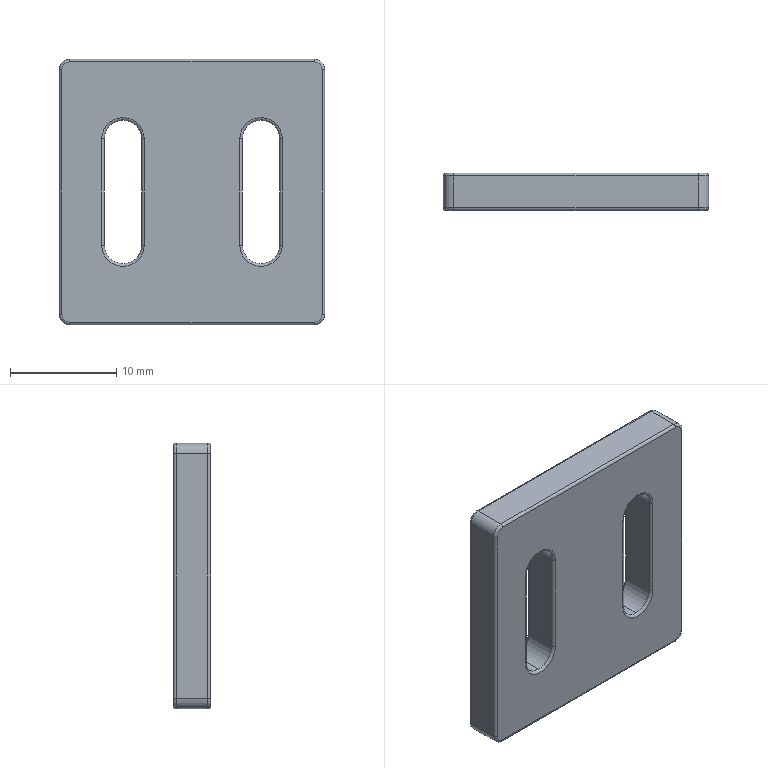Part | SolidWorks | features Extrusion 1, Fillet 1 | 1 solid | 56 faces | box 25 x 3.5 x 25 mm | volume 1868 mm3 | cylinder 26 | torus 20 | plane 10 | commonest cylinder face diameters 0.5 x16 3.5 x6 2 x4
STEP:
#1=CARTESIAN_POINT('',(-6.5,3.5,7.));
#2=VERTEX_POINT('',#1);
#3=CARTESIAN_POINT('',(-8.5,3.5,5.));
#4=VERTEX_POINT('',#3);
#5=CARTESIAN_POINT('',(-6.5,3.5,5.));
#6=DIRECTION('',(0.,-1.,0.));
#7=DIRECTION('',(0.,0.,1.));
#8=AXIS2_PLACEMENT_3D('',#5,#6,#7);
#9=CIRCLE('',#8,2.);
#10=EDGE_CURVE('',#2,#4,#9,.T.);
#11=ORIENTED_EDGE('',*,*,#10,.F.);
#12=CARTESIAN_POINT('',(-6.5,3.25,6.75));
#13=VERTEX_POINT('',#12);
#14=CARTESIAN_POINT('',(-6.5,3.25,7.));
#15=DIRECTION('',(-1.,0.,0.));
#16=DIRECTION('',(0.,0.,1.));
#17=AXIS2_PLACEMENT_3D('',#14,#15,#16);
#18=CIRCLE('',#17,0.25);
#19=EDGE_CURVE('',#2,#13,#18,.T.);
#20=ORIENTED_EDGE('',*,*,#19,.T.);
#21=CARTESIAN_POINT('',(-8.25,3.25,5.));
#22=VERTEX_POINT('',#21);
#23=CARTESIAN_POINT('',(-6.5,3.25,5.));
#24=DIRECTION('',(0.,1.,0.));
#25=DIRECTION('',(0.,0.,1.));
#26=AXIS2_PLACEMENT_3D('',#23,#24,#25);
#27=CIRCLE('',#26,1.75);
#28=EDGE_CURVE('',#22,#13,#27,.T.);
#29=ORIENTED_EDGE('',*,*,#28,.F.);
#30=CARTESIAN_POINT('',(-8.5,3.25,5.));
#31=DIRECTION('',(0.,0.,-1.));
#32=DIRECTION('',(-1.,0.,0.));
#33=AXIS2_PLACEMENT_3D('',#30,#31,#32);
#34=CIRCLE('',#33,0.25);
#35=EDGE_CURVE('',#4,#22,#34,.T.);
#36=ORIENTED_EDGE('',*,*,#35,.F.);
#37=EDGE_LOOP('',(#11,#20,#29,#36));
#38=FACE_OUTER_BOUND('',#37,.T.);
#39=CARTESIAN_POINT('',(-6.5,3.25,5.));
#40=DIRECTION('',(0.,1.,0.));
#41=DIRECTION('',(0.,0.,1.));
#42=AXIS2_PLACEMENT_3D('',#39,#40,#41);
#43=TOROIDAL_SURFACE('',#42,2.,0.25);
#44=ADVANCED_FACE('',(#38),#43,.T.);
#45=CARTESIAN_POINT('',(6.5,3.5,7.));
#46=VERTEX_POINT('',#45);
#47=CARTESIAN_POINT('',(4.5,3.5,5.));
#48=VERTEX_POINT('',#47);
#49=CARTESIAN_POINT('',(6.5,3.5,5.));
#50=DIRECTION('',(0.,-1.,0.));
#51=DIRECTION('',(0.,0.,1.));
#52=AXIS2_PLACEMENT_3D('',#49,#50,#51);
#53=CIRCLE('',#52,2.);
#54=EDGE_CURVE('',#46,#48,#53,.T.);
#55=ORIENTED_EDGE('',*,*,#54,.F.);
#56=CARTESIAN_POINT('',(6.5,3.25,6.75));
#57=VERTEX_POINT('',#56);
#58=CARTESIAN_POINT('',(6.5,3.25,7.));
#59=DIRECTION('',(-1.,0.,0.));
#60=DIRECTION('',(0.,0.,1.));
#61=AXIS2_PLACEMENT_3D('',#58,#59,#60);
#62=CIRCLE('',#61,0.25);
#63=EDGE_CURVE('',#46,#57,#62,.T.);
#64=ORIENTED_EDGE('',*,*,#63,.T.);
#65=CARTESIAN_POINT('',(4.75,3.25,5.));
#66=VERTEX_POINT('',#65);
#67=CARTESIAN_POINT('',(6.5,3.25,5.));
#68=DIRECTION('',(0.,1.,0.));
#69=DIRECTION('',(0.,0.,1.));
#70=AXIS2_PLACEMENT_3D('',#67,#68,#69);
#71=CIRCLE('',#70,1.75);
#72=EDGE_CURVE('',#66,#57,#71,.T.);
#73=ORIENTED_EDGE('',*,*,#72,.F.);
#74=CARTESIAN_POINT('',(4.5,3.25,5.));
#75=DIRECTION('',(0.,0.,-1.));
#76=DIRECTION('',(-1.,0.,0.));
#77=AXIS2_PLACEMENT_3D('',#74,#75,#76);
#78=CIRCLE('',#77,0.25);
#79=EDGE_CURVE('',#48,#66,#78,.T.);
#80=ORIENTED_EDGE('',*,*,#79,.F.);
#81=EDGE_LOOP('',(#55,#64,#73,#80));
#82=FACE_OUTER_BOUND('',#81,.T.);
#83=CARTESIAN_POINT('',(6.5,3.25,5.));
#84=DIRECTION('',(0.,1.,0.));
#85=DIRECTION('',(0.,0.,1.));
#86=AXIS2_PLACEMENT_3D('',#83,#84,#85);
#87=TOROIDAL_SURFACE('',#86,2.,0.25);
#88=ADVANCED_FACE('',(#82),#87,.T.);
#89=CARTESIAN_POINT('',(-6.5,0.25,6.75));
#90=VERTEX_POINT('',#89);
#91=CARTESIAN_POINT('',(-8.25,0.25,5.));
#92=VERTEX_POINT('',#91);
#93=CARTESIAN_POINT('',(-6.5,0.25,5.));
#94=DIRECTION('',(0.,-1.,0.));
#95=DIRECTION('',(0.,0.,1.));
#96=AXIS2_PLACEMENT_3D('',#93,#94,#95);
#97=CIRCLE('',#96,1.75);
#98=EDGE_CURVE('',#90,#92,#97,.T.);
#99=ORIENTED_EDGE('',*,*,#98,.F.);
#100=CARTESIAN_POINT('',(-6.5,0.,7.));
#101=VERTEX_POINT('',#100);
#102=CARTESIAN_POINT('',(-6.5,0.25,7.));
#103=DIRECTION('',(-1.,0.,0.));
#104=DIRECTION('',(0.,0.,1.));
#105=AXIS2_PLACEMENT_3D('',#102,#103,#104);
#106=CIRCLE('',#105,0.25);
#107=EDGE_CURVE('',#90,#101,#106,.T.);
#108=ORIENTED_EDGE('',*,*,#107,.T.);
#109=CARTESIAN_POINT('',(-8.5,0.,5.));
#110=VERTEX_POINT('',#109);
#111=CARTESIAN_POINT('',(-6.5,0.,5.));
#112=DIRECTION('',(0.,1.,0.));
#113=DIRECTION('',(0.,0.,1.));
#114=AXIS2_PLACEMENT_3D('',#111,#112,#113);
#115=CIRCLE('',#114,2.);
#116=EDGE_CURVE('',#110,#101,#115,.T.);
#117=ORIENTED_EDGE('',*,*,#116,.F.);
#118=CARTESIAN_POINT('',(-8.5,0.25,5.));
#119=DIRECTION('',(0.,0.,-1.));
#120=DIRECTION('',(-1.,0.,0.));
#121=AXIS2_PLACEMENT_3D('',#118,#119,#120);
#122=CIRCLE('',#121,0.25);
#123=EDGE_CURVE('',#92,#110,#122,.T.);
#124=ORIENTED_EDGE('',*,*,#123,.F.);
#125=EDGE_LOOP('',(#99,#108,#117,#124));
#126=FACE_OUTER_BOUND('',#125,.T.);
#127=CARTESIAN_POINT('',(-6.5,0.25,5.));
#128=DIRECTION('',(0.,1.,0.));
#129=DIRECTION('',(0.,0.,1.));
#130=AXIS2_PLACEMENT_3D('',#127,#128,#129);
#131=TOROIDAL_SURFACE('',#130,2.,0.25);
#132=ADVANCED_FACE('',(#126),#131,.T.);
#133=CARTESIAN_POINT('',(6.5,0.25,6.75));
#134=VERTEX_POINT('',#133);
#135=CARTESIAN_POINT('',(4.75,0.25,5.));
#136=VERTEX_POINT('',#135);
#137=CARTESIAN_POINT('',(6.5,0.25,5.));
#138=DIRECTION('',(0.,-1.,0.));
#139=DIRECTION('',(0.,0.,1.));
#140=AXIS2_PLACEMENT_3D('',#137,#138,#139);
#141=CIRCLE('',#140,1.75);
#142=EDGE_CURVE('',#134,#136,#141,.T.);
#143=ORIENTED_EDGE('',*,*,#142,.F.);
#144=CARTESIAN_POINT('',(6.5,0.,7.));
#145=VERTEX_POINT('',#144);
#146=CARTESIAN_POINT('',(6.5,0.25,7.));
#147=DIRECTION('',(-1.,0.,0.));
#148=DIRECTION('',(0.,0.,1.));
#149=AXIS2_PLACEMENT_3D('',#146,#147,#148);
#150=CIRCLE('',#149,0.25);
#151=EDGE_CURVE('',#134,#145,#150,.T.);
#152=ORIENTED_EDGE('',*,*,#151,.T.);
#153=CARTESIAN_POINT('',(4.5,0.,5.));
#154=VERTEX_POINT('',#153);
#155=CARTESIAN_POINT('',(6.5,0.,5.));
#156=DIRECTION('',(0.,1.,0.));
#157=DIRECTION('',(0.,0.,1.));
#158=AXIS2_PLACEMENT_3D('',#155,#156,#157);
#159=CIRCLE('',#158,2.);
#160=EDGE_CURVE('',#154,#145,#159,.T.);
#161=ORIENTED_EDGE('',*,*,#160,.F.);
#162=CARTESIAN_POINT('',(4.5,0.25,5.));
#163=DIRECTION('',(0.,0.,-1.));
#164=DIRECTION('',(-1.,0.,0.));
#165=AXIS2_PLACEMENT_3D('',#162,#163,#164);
#166=CIRCLE('',#165,0.25);
#167=EDGE_CURVE('',#136,#154,#166,.T.);
#168=ORIENTED_EDGE('',*,*,#167,.F.);
#169=EDGE_LOOP('',(#143,#152,#161,#168));
#170=FACE_OUTER_BOUND('',#169,.T.);
#171=CARTESIAN_POINT('',(6.5,0.25,5.));
#172=DIRECTION('',(0.,1.,0.));
#173=DIRECTION('',(0.,0.,1.));
#174=AXIS2_PLACEMENT_3D('',#171,#172,#173);
#175=TOROIDAL_SURFACE('',#174,2.,0.25);
#176=ADVANCED_FACE('',(#170),#175,.T.);
#177=CARTESIAN_POINT('',(8.25,3.25,-5.));
#178=VERTEX_POINT('',#177);
#179=CARTESIAN_POINT('',(6.5,3.25,-6.75));
#180=VERTEX_POINT('',#179);
#181=CARTESIAN_POINT('',(6.5,3.25,-5.));
#182=DIRECTION('',(0.,1.,0.));
#183=DIRECTION('',(0.,0.,1.));
#184=AXIS2_PLACEMENT_3D('',#181,#182,#183);
#185=CIRCLE('',#184,1.75);
#186=EDGE_CURVE('',#178,#180,#185,.T.);
#187=ORIENTED_EDGE('',*,*,#186,.T.);
#188=CARTESIAN_POINT('',(6.5,0.25,-6.75));
#189=VERTEX_POINT('',#188);
#190=CARTESIAN_POINT('',(6.5,3.5,-6.75));
#191=DIRECTION('',(0.,-1.,0.));
#192=VECTOR('',#191,1000.);
#193=LINE('',#190,#192);
#194=EDGE_CURVE('',#180,#189,#193,.T.);
#195=ORIENTED_EDGE('',*,*,#194,.T.);
#196=CARTESIAN_POINT('',(8.25,0.25,-5.));
#197=VERTEX_POINT('',#196);
#198=CARTESIAN_POINT('',(6.5,0.25,-5.));
#199=DIRECTION('',(0.,-1.,0.));
#200=DIRECTION('',(0.,0.,1.));
#201=AXIS2_PLACEMENT_3D('',#198,#199,#200);
#202=CIRCLE('',#201,1.75);
#203=EDGE_CURVE('',#189,#197,#202,.T.);
#204=ORIENTED_EDGE('',*,*,#203,.T.);
#205=CARTESIAN_POINT('',(8.25,3.5,-5.));
#206=DIRECTION('',(0.,-1.,0.));
#207=VECTOR('',#206,1000.);
#208=LINE('',#205,#207);
#209=EDGE_CURVE('',#178,#197,#208,.T.);
#210=ORIENTED_EDGE('',*,*,#209,.F.);
#211=EDGE_LOOP('',(#187,#195,#204,#210));
#212=FACE_OUTER_BOUND('',#211,.T.);
#213=CARTESIAN_POINT('',(6.5,3.5,-5.));
#214=DIRECTION('',(0.,-1.,0.));
#215=DIRECTION('',(0.,0.,-1.));
#216=AXIS2_PLACEMENT_3D('',#213,#214,#215);
#217=CYLINDRICAL_SURFACE('',#216,1.75);
#218=ADVANCED_FACE('',(#212),#217,.F.);
#219=CARTESIAN_POINT('',(-4.75,3.25,-5.));
#220=VERTEX_POINT('',#219);
#221=CARTESIAN_POINT('',(-6.5,3.25,-6.75));
#222=VERTEX_POINT('',#221);
#223=CARTESIAN_POINT('',(-6.5,3.25,-5.));
#224=DIRECTION('',(0.,1.,0.));
#225=DIRECTION('',(0.,0.,1.));
#226=AXIS2_PLACEMENT_3D('',#223,#224,#225);
#227=CIRCLE('',#226,1.75);
#228=EDGE_CURVE('',#220,#222,#227,.T.);
#229=ORIENTED_EDGE('',*,*,#228,.T.);
#230=CARTESIAN_POINT('',(-6.5,0.25,-6.75));
#231=VERTEX_POINT('',#230);
#232=CARTESIAN_POINT('',(-6.5,3.5,-6.75));
#233=DIRECTION('',(0.,-1.,0.));
#234=VECTOR('',#233,1000.);
#235=LINE('',#232,#234);
#236=EDGE_CURVE('',#222,#231,#235,.T.);
#237=ORIENTED_EDGE('',*,*,#236,.T.);
#238=CARTESIAN_POINT('',(-4.75,0.25,-5.));
#239=VERTEX_POINT('',#238);
#240=CARTESIAN_POINT('',(-6.5,0.25,-5.));
#241=DIRECTION('',(0.,-1.,0.));
#242=DIRECTION('',(0.,0.,1.));
#243=AXIS2_PLACEMENT_3D('',#240,#241,#242);
#244=CIRCLE('',#243,1.75);
#245=EDGE_CURVE('',#231,#239,#244,.T.);
#246=ORIENTED_EDGE('',*,*,#245,.T.);
#247=CARTESIAN_POINT('',(-4.75,3.5,-5.));
#248=DIRECTION('',(0.,-1.,0.));
#249=VECTOR('',#248,1000.);
#250=LINE('',#247,#249);
#251=EDGE_CURVE('',#220,#239,#250,.T.);
#252=ORIENTED_EDGE('',*,*,#251,.F.);
#253=EDGE_LOOP('',(#229,#237,#246,#252));
#254=FACE_OUTER_BOUND('',#253,.T.);
#255=CARTESIAN_POINT('',(-6.5,3.5,-5.));
#256=DIRECTION('',(0.,-1.,0.));
#257=DIRECTION('',(0.,0.,-1.));
#258=AXIS2_PLACEMENT_3D('',#255,#256,#257);
#259=CYLINDRICAL_SURFACE('',#258,1.75);
#260=ADVANCED_FACE('',(#254),#259,.F.);
#261=CARTESIAN_POINT('',(4.5,3.5,-5.));
#262=VERTEX_POINT('',#261);
#263=CARTESIAN_POINT('',(4.5,3.5,-11.5));
#264=DIRECTION('',(0.,0.,-1.));
#265=VECTOR('',#264,1000.);
#266=LINE('',#263,#265);
#267=EDGE_CURVE('',#48,#262,#266,.T.);
#268=ORIENTED_EDGE('',*,*,#267,.T.);
#269=CARTESIAN_POINT('',(8.5,3.5,-5.));
#270=VERTEX_POINT('',#269);
#271=CARTESIAN_POINT('',(6.5,3.5,-5.));
#272=DIRECTION('',(0.,-1.,0.));
#273=DIRECTION('',(0.,0.,1.));
#274=AXIS2_PLACEMENT_3D('',#271,#272,#273);
#275=CIRCLE('',#274,2.);
#276=EDGE_CURVE('',#262,#270,#275,.T.);
#277=ORIENTED_EDGE('',*,*,#276,.T.);
#278=CARTESIAN_POINT('',(8.5,3.5,5.));
#279=VERTEX_POINT('',#278);
#280=CARTESIAN_POINT('',(8.5,3.5,-11.5));
#281=DIRECTION('',(0.,0.,1.));
#282=VECTOR('',#281,1000.);
#283=LINE('',#280,#282);
#284=EDGE_CURVE('',#270,#279,#283,.T.);
#285=ORIENTED_EDGE('',*,*,#284,.T.);
#286=CARTESIAN_POINT('',(6.5,3.5,5.));
#287=DIRECTION('',(0.,-1.,0.));
#288=DIRECTION('',(0.,0.,1.));
#289=AXIS2_PLACEMENT_3D('',#286,#287,#288);
#290=CIRCLE('',#289,2.);
#291=EDGE_CURVE('',#279,#46,#290,.T.);
#292=ORIENTED_EDGE('',*,*,#291,.T.);
#293=ORIENTED_EDGE('',*,*,#54,.T.);
#294=EDGE_LOOP('',(#268,#277,#285,#292,#293));
#295=FACE_BOUND('',#294,.T.);
#296=CARTESIAN_POINT('',(-8.5,3.5,-5.));
#297=VERTEX_POINT('',#296);
#298=CARTESIAN_POINT('',(-8.5,3.5,-11.5));
#299=DIRECTION('',(0.,0.,-1.));
#300=VECTOR('',#299,1000.);
#301=LINE('',#298,#300);
#302=EDGE_CURVE('',#4,#297,#301,.T.);
#303=ORIENTED_EDGE('',*,*,#302,.T.);
#304=CARTESIAN_POINT('',(-4.5,3.5,-5.));
#305=VERTEX_POINT('',#304);
#306=CARTESIAN_POINT('',(-6.5,3.5,-5.));
#307=DIRECTION('',(0.,-1.,0.));
#308=DIRECTION('',(0.,0.,1.));
#309=AXIS2_PLACEMENT_3D('',#306,#307,#308);
#310=CIRCLE('',#309,2.);
#311=EDGE_CURVE('',#297,#305,#310,.T.);
#312=ORIENTED_EDGE('',*,*,#311,.T.);
#313=CARTESIAN_POINT('',(-4.5,3.5,5.));
#314=VERTEX_POINT('',#313);
#315=CARTESIAN_POINT('',(-4.5,3.5,-11.5));
#316=DIRECTION('',(0.,0.,1.));
#317=VECTOR('',#316,1000.);
#318=LINE('',#315,#317);
#319=EDGE_CURVE('',#305,#314,#318,.T.);
#320=ORIENTED_EDGE('',*,*,#319,.T.);
#321=CARTESIAN_POINT('',(-6.5,3.5,5.));
#322=DIRECTION('',(0.,-1.,0.));
#323=DIRECTION('',(0.,0.,1.));
#324=AXIS2_PLACEMENT_3D('',#321,#322,#323);
#325=CIRCLE('',#324,2.);
#326=EDGE_CURVE('',#314,#2,#325,.T.);
#327=ORIENTED_EDGE('',*,*,#326,.T.);
#328=ORIENTED_EDGE('',*,*,#10,.T.);
#329=EDGE_LOOP('',(#303,#312,#320,#327,#328));
#330=FACE_BOUND('',#329,.T.);
#331=CARTESIAN_POINT('',(12.25,3.5,-11.5));
#332=VERTEX_POINT('',#331);
#333=CARTESIAN_POINT('',(11.5,3.5,-12.25));
#334=VERTEX_POINT('',#333);
#335=CARTESIAN_POINT('',(11.5,3.5,-11.5));
#336=DIRECTION('',(0.,1.,0.));
#337=DIRECTION('',(0.,0.,1.));
#338=AXIS2_PLACEMENT_3D('',#335,#336,#337);
#339=CIRCLE('',#338,0.75);
#340=EDGE_CURVE('',#332,#334,#339,.T.);
#341=ORIENTED_EDGE('',*,*,#340,.T.);
#342=CARTESIAN_POINT('',(-11.5,3.5,-12.25));
#343=VERTEX_POINT('',#342);
#344=CARTESIAN_POINT('',(-11.5,3.5,-12.25));
#345=DIRECTION('',(-1.,0.,0.));
#346=VECTOR('',#345,1000.);
#347=LINE('',#344,#346);
#348=EDGE_CURVE('',#334,#343,#347,.T.);
#349=ORIENTED_EDGE('',*,*,#348,.T.);
#350=CARTESIAN_POINT('',(-12.25,3.5,-11.5));
#351=VERTEX_POINT('',#350);
#352=CARTESIAN_POINT('',(-11.5,3.5,-11.5));
#353=DIRECTION('',(0.,1.,0.));
#354=DIRECTION('',(0.,0.,1.));
#355=AXIS2_PLACEMENT_3D('',#352,#353,#354);
#356=CIRCLE('',#355,0.75);
#357=EDGE_CURVE('',#343,#351,#356,.T.);
#358=ORIENTED_EDGE('',*,*,#357,.T.);
#359=CARTESIAN_POINT('',(-12.25,3.5,11.5));
#360=VERTEX_POINT('',#359);
#361=CARTESIAN_POINT('',(-12.25,3.5,11.5));
#362=DIRECTION('',(0.,0.,1.));
#363=VECTOR('',#362,1000.);
#364=LINE('',#361,#363);
#365=EDGE_CURVE('',#351,#360,#364,.T.);
#366=ORIENTED_EDGE('',*,*,#365,.T.);
#367=CARTESIAN_POINT('',(-11.5,3.5,12.25));
#368=VERTEX_POINT('',#367);
#369=CARTESIAN_POINT('',(-11.5,3.5,11.5));
#370=DIRECTION('',(0.,1.,0.));
#371=DIRECTION('',(0.,0.,1.));
#372=AXIS2_PLACEMENT_3D('',#369,#370,#371);
#373=CIRCLE('',#372,0.75);
#374=EDGE_CURVE('',#360,#368,#373,.T.);
#375=ORIENTED_EDGE('',*,*,#374,.T.);
#376=CARTESIAN_POINT('',(11.5,3.5,12.25));
#377=VERTEX_POINT('',#376);
#378=CARTESIAN_POINT('',(11.5,3.5,12.25));
#379=DIRECTION('',(1.,0.,0.));
#380=VECTOR('',#379,1000.);
#381=LINE('',#378,#380);
#382=EDGE_CURVE('',#368,#377,#381,.T.);
#383=ORIENTED_EDGE('',*,*,#382,.T.);
#384=CARTESIAN_POINT('',(12.25,3.5,11.5));
#385=VERTEX_POINT('',#384);
#386=CARTESIAN_POINT('',(11.5,3.5,11.5));
#387=DIRECTION('',(0.,1.,0.));
#388=DIRECTION('',(0.,0.,1.));
#389=AXIS2_PLACEMENT_3D('',#386,#387,#388);
#390=CIRCLE('',#389,0.75);
#391=EDGE_CURVE('',#377,#385,#390,.T.);
#392=ORIENTED_EDGE('',*,*,#391,.T.);
#393=CARTESIAN_POINT('',(12.25,3.5,-11.5));
#394=DIRECTION('',(0.,0.,-1.));
#395=VECTOR('',#394,1000.);
#396=LINE('',#393,#395);
#397=EDGE_CURVE('',#385,#332,#396,.T.);
#398=ORIENTED_EDGE('',*,*,#397,.T.);
#399=EDGE_LOOP('',(#341,#349,#358,#366,#375,#383,#392,#398));
#400=FACE_OUTER_BOUND('',#399,.T.);
#401=CARTESIAN_POINT('',(-11.5,3.5,-11.5));
#402=DIRECTION('',(0.,1.,0.));
#403=DIRECTION('',(0.,0.,1.));
#404=AXIS2_PLACEMENT_3D('',#401,#402,#403);
#405=PLANE('',#404);
#406=ADVANCED_FACE('',(#295,#330,#400),#405,.T.);
#407=CARTESIAN_POINT('',(8.5,0.,-5.));
#408=VERTEX_POINT('',#407);
#409=CARTESIAN_POINT('',(4.5,0.,-5.));
#410=VERTEX_POINT('',#409);
#411=CARTESIAN_POINT('',(6.5,0.,-5.));
#412=DIRECTION('',(0.,1.,0.));
#413=DIRECTION('',(0.,0.,1.));
#414=AXIS2_PLACEMENT_3D('',#411,#412,#413);
#415=CIRCLE('',#414,2.);
#416=EDGE_CURVE('',#408,#410,#415,.T.);
#417=ORIENTED_EDGE('',*,*,#416,.T.);
#418=CARTESIAN_POINT('',(4.5,0.,5.));
#419=DIRECTION('',(0.,0.,1.));
#420=VECTOR('',#419,1000.);
#421=LINE('',#418,#420);
#422=EDGE_CURVE('',#410,#154,#421,.T.);
#423=ORIENTED_EDGE('',*,*,#422,.T.);
#424=ORIENTED_EDGE('',*,*,#160,.T.);
#425=CARTESIAN_POINT('',(8.5,0.,5.));
#426=VERTEX_POINT('',#425);
#427=CARTESIAN_POINT('',(6.5,0.,5.));
#428=DIRECTION('',(0.,1.,0.));
#429=DIRECTION('',(0.,0.,1.));
#430=AXIS2_PLACEMENT_3D('',#427,#428,#429);
#431=CIRCLE('',#430,2.);
#432=EDGE_CURVE('',#145,#426,#431,.T.);
#433=ORIENTED_EDGE('',*,*,#432,.T.);
#434=CARTESIAN_POINT('',(8.5,0.,-5.));
#435=DIRECTION('',(0.,0.,-1.));
#436=VECTOR('',#435,1000.);
#437=LINE('',#434,#436);
#438=EDGE_CURVE('',#426,#408,#437,.T.);
#439=ORIENTED_EDGE('',*,*,#438,.T.);
#440=EDGE_LOOP('',(#417,#423,#424,#433,#439));
#441=FACE_BOUND('',#440,.T.);
#442=CARTESIAN_POINT('',(-11.5,0.,12.25));
#443=VERTEX_POINT('',#442);
#444=CARTESIAN_POINT('',(-12.25,0.,11.5));
#445=VERTEX_POINT('',#444);
#446=CARTESIAN_POINT('',(-11.5,0.,11.5));
#447=DIRECTION('',(0.,-1.,0.));
#448=DIRECTION('',(0.,0.,1.));
#449=AXIS2_PLACEMENT_3D('',#446,#447,#448);
#450=CIRCLE('',#449,0.75);
#451=EDGE_CURVE('',#443,#445,#450,.T.);
#452=ORIENTED_EDGE('',*,*,#451,.T.);
#453=CARTESIAN_POINT('',(-12.25,0.,-11.5));
#454=VERTEX_POINT('',#453);
#455=CARTESIAN_POINT('',(-12.25,0.,-11.5));
#456=DIRECTION('',(0.,0.,-1.));
#457=VECTOR('',#456,1000.);
#458=LINE('',#455,#457);
#459=EDGE_CURVE('',#445,#454,#458,.T.);
#460=ORIENTED_EDGE('',*,*,#459,.T.);
#461=CARTESIAN_POINT('',(-11.5,0.,-12.25));
#462=VERTEX_POINT('',#461);
#463=CARTESIAN_POINT('',(-11.5,0.,-11.5));
#464=DIRECTION('',(0.,-1.,0.));
#465=DIRECTION('',(0.,0.,1.));
#466=AXIS2_PLACEMENT_3D('',#463,#464,#465);
#467=CIRCLE('',#466,0.75);
#468=EDGE_CURVE('',#454,#462,#467,.T.);
#469=ORIENTED_EDGE('',*,*,#468,.T.);
#470=CARTESIAN_POINT('',(11.5,0.,-12.25));
#471=VERTEX_POINT('',#470);
#472=CARTESIAN_POINT('',(-11.5,0.,-12.25));
#473=DIRECTION('',(1.,0.,0.));
#474=VECTOR('',#473,1000.);
#475=LINE('',#472,#474);
#476=EDGE_CURVE('',#462,#471,#475,.T.);
#477=ORIENTED_EDGE('',*,*,#476,.T.);
#478=CARTESIAN_POINT('',(12.25,0.,-11.5));
#479=VERTEX_POINT('',#478);
#480=CARTESIAN_POINT('',(11.5,0.,-11.5));
#481=DIRECTION('',(0.,-1.,0.));
#482=DIRECTION('',(0.,0.,1.));
#483=AXIS2_PLACEMENT_3D('',#480,#481,#482);
#484=CIRCLE('',#483,0.75);
#485=EDGE_CURVE('',#471,#479,#484,.T.);
#486=ORIENTED_EDGE('',*,*,#485,.T.);
#487=CARTESIAN_POINT('',(12.25,0.,11.5));
#488=VERTEX_POINT('',#487);
#489=CARTESIAN_POINT('',(12.25,0.,-11.5));
#490=DIRECTION('',(0.,0.,1.));
#491=VECTOR('',#490,1000.);
#492=LINE('',#489,#491);
#493=EDGE_CURVE('',#479,#488,#492,.T.);
#494=ORIENTED_EDGE('',*,*,#493,.T.);
#495=CARTESIAN_POINT('',(11.5,0.,12.25));
#496=VERTEX_POINT('',#495);
#497=CARTESIAN_POINT('',(11.5,0.,11.5));
#498=DIRECTION('',(0.,-1.,0.));
#499=DIRECTION('',(0.,0.,1.));
#500=AXIS2_PLACEMENT_3D('',#497,#498,#499);
#501=CIRCLE('',#500,0.75);
#502=EDGE_CURVE('',#488,#496,#501,.T.);
#503=ORIENTED_EDGE('',*,*,#502,.T.);
#504=CARTESIAN_POINT('',(-11.5,0.,12.25));
#505=DIRECTION('',(-1.,0.,0.));
#506=VECTOR('',#505,1000.);
#507=LINE('',#504,#506);
#508=EDGE_CURVE('',#496,#443,#507,.T.);
#509=ORIENTED_EDGE('',*,*,#508,.T.);
#510=EDGE_LOOP('',(#452,#460,#469,#477,#486,#494,#503,#509));
#511=FACE_OUTER_BOUND('',#510,.T.);
#512=CARTESIAN_POINT('',(-4.5,0.,-5.));
#513=VERTEX_POINT('',#512);
#514=CARTESIAN_POINT('',(-8.5,0.,-5.));
#515=VERTEX_POINT('',#514);
#516=CARTESIAN_POINT('',(-6.5,0.,-5.));
#517=DIRECTION('',(0.,1.,0.));
#518=DIRECTION('',(0.,0.,1.));
#519=AXIS2_PLACEMENT_3D('',#516,#517,#518);
#520=CIRCLE('',#519,2.);
#521=EDGE_CURVE('',#513,#515,#520,.T.);
#522=ORIENTED_EDGE('',*,*,#521,.T.);
#523=CARTESIAN_POINT('',(-8.5,0.,5.));
#524=DIRECTION('',(0.,0.,1.));
#525=VECTOR('',#524,1000.);
#526=LINE('',#523,#525);
#527=EDGE_CURVE('',#515,#110,#526,.T.);
#528=ORIENTED_EDGE('',*,*,#527,.T.);
#529=ORIENTED_EDGE('',*,*,#116,.T.);
#530=CARTESIAN_POINT('',(-4.5,0.,5.));
#531=VERTEX_POINT('',#530);
#532=CARTESIAN_POINT('',(-6.5,0.,5.));
#533=DIRECTION('',(0.,1.,0.));
#534=DIRECTION('',(0.,0.,1.));
#535=AXIS2_PLACEMENT_3D('',#532,#533,#534);
#536=CIRCLE('',#535,2.);
#537=EDGE_CURVE('',#101,#531,#536,.T.);
#538=ORIENTED_EDGE('',*,*,#537,.T.);
#539=CARTESIAN_POINT('',(-4.5,0.,-5.));
#540=DIRECTION('',(0.,0.,-1.));
#541=VECTOR('',#540,1000.);
#542=LINE('',#539,#541);
#543=EDGE_CURVE('',#531,#513,#542,.T.);
#544=ORIENTED_EDGE('',*,*,#543,.T.);
#545=EDGE_LOOP('',(#522,#528,#529,#538,#544));
#546=FACE_BOUND('',#545,.T.);
#547=CARTESIAN_POINT('',(-11.5,0.,-11.5));
#548=DIRECTION('',(0.,1.,0.));
#549=DIRECTION('',(0.,0.,1.));
#550=AXIS2_PLACEMENT_3D('',#547,#548,#549);
#551=PLANE('',#550);
#552=ADVANCED_FACE('',(#441,#511,#546),#551,.F.);
#553=CARTESIAN_POINT('',(-11.5,3.25,-12.5));
#554=VERTEX_POINT('',#553);
#555=CARTESIAN_POINT('',(-11.5,0.25,-12.5));
#556=VERTEX_POINT('',#555);
#557=CARTESIAN_POINT('',(-11.5,3.5,-12.5));
#558=DIRECTION('',(0.,-1.,0.));
#559=VECTOR('',#558,1000.);
#560=LINE('',#557,#559);
#561=EDGE_CURVE('',#554,#556,#560,.T.);
#562=ORIENTED_EDGE('',*,*,#561,.T.);
#563=CARTESIAN_POINT('',(-12.5,0.25,-11.5));
#564=VERTEX_POINT('',#563);
#565=CARTESIAN_POINT('',(-11.5,0.25,-11.5));
#566=DIRECTION('',(0.,1.,0.));
#567=DIRECTION('',(0.,0.,1.));
#568=AXIS2_PLACEMENT_3D('',#565,#566,#567);
#569=CIRCLE('',#568,1.);
#570=EDGE_CURVE('',#556,#564,#569,.T.);
#571=ORIENTED_EDGE('',*,*,#570,.T.);
#572=CARTESIAN_POINT('',(-12.5,3.25,-11.5));
#573=VERTEX_POINT('',#572);
#574=CARTESIAN_POINT('',(-12.5,3.5,-11.5));
#575=DIRECTION('',(0.,-1.,0.));
#576=VECTOR('',#575,1000.);
#577=LINE('',#574,#576);
#578=EDGE_CURVE('',#573,#564,#577,.T.);
#579=ORIENTED_EDGE('',*,*,#578,.F.);
#580=CARTESIAN_POINT('',(-11.5,3.25,-11.5));
#581=DIRECTION('',(0.,-1.,0.));
#582=DIRECTION('',(0.,0.,1.));
#583=AXIS2_PLACEMENT_3D('',#580,#581,#582);
#584=CIRCLE('',#583,1.);
#585=EDGE_CURVE('',#573,#554,#584,.T.);
#586=ORIENTED_EDGE('',*,*,#585,.T.);
#587=EDGE_LOOP('',(#562,#571,#579,#586));
#588=FACE_OUTER_BOUND('',#587,.T.);
#589=CARTESIAN_POINT('',(-11.5,3.5,-11.5));
#590=DIRECTION('',(0.,-1.,0.));
#591=DIRECTION('',(0.,0.,-1.));
#592=AXIS2_PLACEMENT_3D('',#589,#590,#591);
#593=CYLINDRICAL_SURFACE('',#592,1.);
#594=ADVANCED_FACE('',(#588),#593,.T.);
#595=ORIENTED_EDGE('',*,*,#578,.T.);
#596=CARTESIAN_POINT('',(-12.5,0.25,11.5));
#597=VERTEX_POINT('',#596);
#598=CARTESIAN_POINT('',(-12.5,0.25,-11.5));
#599=DIRECTION('',(0.,0.,1.));
#600=VECTOR('',#599,1000.);
#601=LINE('',#598,#600);
#602=EDGE_CURVE('',#564,#597,#601,.T.);
#603=ORIENTED_EDGE('',*,*,#602,.T.);
#604=CARTESIAN_POINT('',(-12.5,3.25,11.5));
#605=VERTEX_POINT('',#604);
#606=CARTESIAN_POINT('',(-12.5,3.5,11.5));
#607=DIRECTION('',(0.,-1.,0.));
#608=VECTOR('',#607,1000.);
#609=LINE('',#606,#608);
#610=EDGE_CURVE('',#605,#597,#609,.T.);
#611=ORIENTED_EDGE('',*,*,#610,.F.);
#612=CARTESIAN_POINT('',(-12.5,3.25,-11.5));
#613=DIRECTION('',(0.,0.,-1.));
#614=VECTOR('',#613,1000.);
#615=LINE('',#612,#614);
#616=EDGE_CURVE('',#605,#573,#615,.T.);
#617=ORIENTED_EDGE('',*,*,#616,.T.);
#618=EDGE_LOOP('',(#595,#603,#611,#617));
#619=FACE_OUTER_BOUND('',#618,.T.);
#620=CARTESIAN_POINT('',(-12.5,3.5,-11.5));
#621=DIRECTION('',(1.,0.,0.));
#622=DIRECTION('',(0.,0.,-1.));
#623=AXIS2_PLACEMENT_3D('',#620,#621,#622);
#624=PLANE('',#623);
#625=ADVANCED_FACE('',(#619),#624,.F.);
#626=ORIENTED_EDGE('',*,*,#610,.T.);
#627=CARTESIAN_POINT('',(-11.5,0.25,12.5));
#628=VERTEX_POINT('',#627);
#629=CARTESIAN_POINT('',(-11.5,0.25,11.5));
#630=DIRECTION('',(0.,1.,0.));
#631=DIRECTION('',(0.,0.,1.));
#632=AXIS2_PLACEMENT_3D('',#629,#630,#631);
#633=CIRCLE('',#632,1.);
#634=EDGE_CURVE('',#597,#628,#633,.T.);
#635=ORIENTED_EDGE('',*,*,#634,.T.);
#636=CARTESIAN_POINT('',(-11.5,3.25,12.5));
#637=VERTEX_POINT('',#636);
#638=CARTESIAN_POINT('',(-11.5,3.5,12.5));
#639=DIRECTION('',(0.,-1.,0.));
#640=VECTOR('',#639,1000.);
#641=LINE('',#638,#640);
#642=EDGE_CURVE('',#637,#628,#641,.T.);
#643=ORIENTED_EDGE('',*,*,#642,.F.);
#644=CARTESIAN_POINT('',(-11.5,3.25,11.5));
#645=DIRECTION('',(0.,-1.,0.));
#646=DIRECTION('',(0.,0.,1.));
#647=AXIS2_PLACEMENT_3D('',#644,#645,#646);
#648=CIRCLE('',#647,1.);
#649=EDGE_CURVE('',#637,#605,#648,.T.);
#650=ORIENTED_EDGE('',*,*,#649,.T.);
#651=EDGE_LOOP('',(#626,#635,#643,#650));
#652=FACE_OUTER_BOUND('',#651,.T.);
#653=CARTESIAN_POINT('',(-11.5,3.5,11.5));
#654=DIRECTION('',(0.,-1.,0.));
#655=DIRECTION('',(0.,0.,-1.));
#656=AXIS2_PLACEMENT_3D('',#653,#654,#655);
#657=CYLINDRICAL_SURFACE('',#656,1.);
#658=ADVANCED_FACE('',(#652),#657,.T.);
#659=ORIENTED_EDGE('',*,*,#642,.T.);
#660=CARTESIAN_POINT('',(11.5,0.25,12.5));
#661=VERTEX_POINT('',#660);
#662=CARTESIAN_POINT('',(-11.5,0.25,12.5));
#663=DIRECTION('',(1.,0.,0.));
#664=VECTOR('',#663,1000.);
#665=LINE('',#662,#664);
#666=EDGE_CURVE('',#628,#661,#665,.T.);
#667=ORIENTED_EDGE('',*,*,#666,.T.);
#668=CARTESIAN_POINT('',(11.5,3.25,12.5));
#669=VERTEX_POINT('',#668);
#670=CARTESIAN_POINT('',(11.5,3.5,12.5));
#671=DIRECTION('',(0.,-1.,0.));
#672=VECTOR('',#671,1000.);
#673=LINE('',#670,#672);
#674=EDGE_CURVE('',#669,#661,#673,.T.);
#675=ORIENTED_EDGE('',*,*,#674,.F.);
#676=CARTESIAN_POINT('',(-11.5,3.25,12.5));
#677=DIRECTION('',(-1.,0.,0.));
#678=VECTOR('',#677,1000.);
#679=LINE('',#676,#678);
#680=EDGE_CURVE('',#669,#637,#679,.T.);
#681=ORIENTED_EDGE('',*,*,#680,.T.);
#682=EDGE_LOOP('',(#659,#667,#675,#681));
#683=FACE_OUTER_BOUND('',#682,.T.);
#684=CARTESIAN_POINT('',(-11.5,3.5,12.5));
#685=DIRECTION('',(0.,0.,-1.));
#686=DIRECTION('',(-1.,0.,0.));
#687=AXIS2_PLACEMENT_3D('',#684,#685,#686);
#688=PLANE('',#687);
#689=ADVANCED_FACE('',(#683),#688,.F.);
#690=ORIENTED_EDGE('',*,*,#674,.T.);
#691=CARTESIAN_POINT('',(12.5,0.25,11.5));
#692=VERTEX_POINT('',#691);
#693=CARTESIAN_POINT('',(11.5,0.25,11.5));
#694=DIRECTION('',(0.,1.,0.));
#695=DIRECTION('',(0.,0.,1.));
#696=AXIS2_PLACEMENT_3D('',#693,#694,#695);
#697=CIRCLE('',#696,1.);
#698=EDGE_CURVE('',#661,#692,#697,.T.);
#699=ORIENTED_EDGE('',*,*,#698,.T.);
#700=CARTESIAN_POINT('',(12.5,3.25,11.5));
#701=VERTEX_POINT('',#700);
#702=CARTESIAN_POINT('',(12.5,3.5,11.5));
#703=DIRECTION('',(0.,-1.,0.));
#704=VECTOR('',#703,1000.);
#705=LINE('',#702,#704);
#706=EDGE_CURVE('',#701,#692,#705,.T.);
#707=ORIENTED_EDGE('',*,*,#706,.F.);
#708=CARTESIAN_POINT('',(11.5,3.25,11.5));
#709=DIRECTION('',(0.,-1.,0.));
#710=DIRECTION('',(0.,0.,1.));
#711=AXIS2_PLACEMENT_3D('',#708,#709,#710);
#712=CIRCLE('',#711,1.);
#713=EDGE_CURVE('',#701,#669,#712,.T.);
#714=ORIENTED_EDGE('',*,*,#713,.T.);
#715=EDGE_LOOP('',(#690,#699,#707,#714));
#716=FACE_OUTER_BOUND('',#715,.T.);
#717=CARTESIAN_POINT('',(11.5,3.5,11.5));
#718=DIRECTION('',(0.,-1.,0.));
#719=DIRECTION('',(0.,0.,-1.));
#720=AXIS2_PLACEMENT_3D('',#717,#718,#719);
#721=CYLINDRICAL_SURFACE('',#720,1.);
#722=ADVANCED_FACE('',(#716),#721,.T.);
#723=ORIENTED_EDGE('',*,*,#706,.T.);
#724=CARTESIAN_POINT('',(12.5,0.25,-11.5));
#725=VERTEX_POINT('',#724);
#726=CARTESIAN_POINT('',(12.5,0.25,-11.5));
#727=DIRECTION('',(0.,0.,-1.));
#728=VECTOR('',#727,1000.);
#729=LINE('',#726,#728);
#730=EDGE_CURVE('',#692,#725,#729,.T.);
#731=ORIENTED_EDGE('',*,*,#730,.T.);
#732=CARTESIAN_POINT('',(12.5,3.25,-11.5));
#733=VERTEX_POINT('',#732);
#734=CARTESIAN_POINT('',(12.5,3.5,-11.5));
#735=DIRECTION('',(0.,-1.,0.));
#736=VECTOR('',#735,1000.);
#737=LINE('',#734,#736);
#738=EDGE_CURVE('',#733,#725,#737,.T.);
#739=ORIENTED_EDGE('',*,*,#738,.F.);
#740=CARTESIAN_POINT('',(12.5,3.25,11.5));
#741=DIRECTION('',(0.,0.,1.));
#742=VECTOR('',#741,1000.);
#743=LINE('',#740,#742);
#744=EDGE_CURVE('',#733,#701,#743,.T.);
#745=ORIENTED_EDGE('',*,*,#744,.T.);
#746=EDGE_LOOP('',(#723,#731,#739,#745));
#747=FACE_OUTER_BOUND('',#746,.T.);
#748=CARTESIAN_POINT('',(12.5,3.5,-11.5));
#749=DIRECTION('',(-1.,0.,0.));
#750=DIRECTION('',(0.,0.,1.));
#751=AXIS2_PLACEMENT_3D('',#748,#749,#750);
#752=PLANE('',#751);
#753=ADVANCED_FACE('',(#747),#752,.F.);
#754=ORIENTED_EDGE('',*,*,#738,.T.);
#755=CARTESIAN_POINT('',(11.5,0.25,-12.5));
#756=VERTEX_POINT('',#755);
#757=CARTESIAN_POINT('',(11.5,0.25,-11.5));
#758=DIRECTION('',(0.,1.,0.));
#759=DIRECTION('',(0.,0.,1.));
#760=AXIS2_PLACEMENT_3D('',#757,#758,#759);
#761=CIRCLE('',#760,1.);
#762=EDGE_CURVE('',#725,#756,#761,.T.);
#763=ORIENTED_EDGE('',*,*,#762,.T.);
#764=CARTESIAN_POINT('',(11.5,3.25,-12.5));
#765=VERTEX_POINT('',#764);
#766=CARTESIAN_POINT('',(11.5,3.5,-12.5));
#767=DIRECTION('',(0.,-1.,0.));
#768=VECTOR('',#767,1000.);
#769=LINE('',#766,#768);
#770=EDGE_CURVE('',#765,#756,#769,.T.);
#771=ORIENTED_EDGE('',*,*,#770,.F.);
#772=CARTESIAN_POINT('',(11.5,3.25,-11.5));
#773=DIRECTION('',(0.,-1.,0.));
#774=DIRECTION('',(0.,0.,1.));
#775=AXIS2_PLACEMENT_3D('',#772,#773,#774);
#776=CIRCLE('',#775,1.);
#777=EDGE_CURVE('',#765,#733,#776,.T.);
#778=ORIENTED_EDGE('',*,*,#777,.T.);
#779=EDGE_LOOP('',(#754,#763,#771,#778));
#780=FACE_OUTER_BOUND('',#779,.T.);
#781=CARTESIAN_POINT('',(11.5,3.5,-11.5));
#782=DIRECTION('',(0.,-1.,0.));
#783=DIRECTION('',(0.,0.,-1.));
#784=AXIS2_PLACEMENT_3D('',#781,#782,#783);
#785=CYLINDRICAL_SURFACE('',#784,1.);
#786=ADVANCED_FACE('',(#780),#785,.T.);
#787=ORIENTED_EDGE('',*,*,#770,.T.);
#788=CARTESIAN_POINT('',(-11.5,0.25,-12.5));
#789=DIRECTION('',(-1.,0.,0.));
#790=VECTOR('',#789,1000.);
#791=LINE('',#788,#790);
#792=EDGE_CURVE('',#756,#556,#791,.T.);
#793=ORIENTED_EDGE('',*,*,#792,.T.);
#794=ORIENTED_EDGE('',*,*,#561,.F.);
#795=CARTESIAN_POINT('',(11.5,3.25,-12.5));
#796=DIRECTION('',(1.,0.,0.));
#797=VECTOR('',#796,1000.);
#798=LINE('',#795,#797);
#799=EDGE_CURVE('',#554,#765,#798,.T.);
#800=ORIENTED_EDGE('',*,*,#799,.T.);
#801=EDGE_LOOP('',(#787,#793,#794,#800));
#802=FACE_OUTER_BOUND('',#801,.T.);
#803=CARTESIAN_POINT('',(-11.5,3.5,-12.5));
#804=DIRECTION('',(0.,0.,1.));
#805=DIRECTION('',(1.,0.,0.));
#806=AXIS2_PLACEMENT_3D('',#803,#804,#805);
#807=PLANE('',#806);
#808=ADVANCED_FACE('',(#802),#807,.F.);
#809=CARTESIAN_POINT('',(-4.75,3.25,5.));
#810=VERTEX_POINT('',#809);
#811=CARTESIAN_POINT('',(-4.75,0.25,5.));
#812=VERTEX_POINT('',#811);
#813=CARTESIAN_POINT('',(-4.75,3.5,5.));
#814=DIRECTION('',(0.,-1.,0.));
#815=VECTOR('',#814,1000.);
#816=LINE('',#813,#815);
#817=EDGE_CURVE('',#810,#812,#816,.T.);
#818=ORIENTED_EDGE('',*,*,#817,.T.);
#819=CARTESIAN_POINT('',(-6.5,0.25,5.));
#820=DIRECTION('',(0.,-1.,0.));
#821=DIRECTION('',(0.,0.,1.));
#822=AXIS2_PLACEMENT_3D('',#819,#820,#821);
#823=CIRCLE('',#822,1.75);
#824=EDGE_CURVE('',#812,#90,#823,.T.);
#825=ORIENTED_EDGE('',*,*,#824,.T.);
#826=ORIENTED_EDGE('',*,*,#98,.T.);
#827=CARTESIAN_POINT('',(-8.25,3.5,5.));
#828=DIRECTION('',(0.,-1.,0.));
#829=VECTOR('',#828,1000.);
#830=LINE('',#827,#829);
#831=EDGE_CURVE('',#22,#92,#830,.T.);
#832=ORIENTED_EDGE('',*,*,#831,.F.);
#833=ORIENTED_EDGE('',*,*,#28,.T.);
#834=CARTESIAN_POINT('',(-6.5,3.25,5.));
#835=DIRECTION('',(0.,1.,0.));
#836=DIRECTION('',(0.,0.,1.));
#837=AXIS2_PLACEMENT_3D('',#834,#835,#836);
#838=CIRCLE('',#837,1.75);
#839=EDGE_CURVE('',#13,#810,#838,.T.);
#840=ORIENTED_EDGE('',*,*,#839,.T.);
#841=EDGE_LOOP('',(#818,#825,#826,#832,#833,#840));
#842=FACE_OUTER_BOUND('',#841,.T.);
#843=CARTESIAN_POINT('',(-6.5,3.5,5.));
#844=DIRECTION('',(0.,-1.,0.));
#845=DIRECTION('',(0.,0.,-1.));
#846=AXIS2_PLACEMENT_3D('',#843,#844,#845);
#847=CYLINDRICAL_SURFACE('',#846,1.75);
#848=ADVANCED_FACE('',(#842),#847,.F.);
#849=ORIENTED_EDGE('',*,*,#251,.T.);
#850=CARTESIAN_POINT('',(-4.75,0.25,5.));
#851=DIRECTION('',(0.,0.,1.));
#852=VECTOR('',#851,1000.);
#853=LINE('',#850,#852);
#854=EDGE_CURVE('',#239,#812,#853,.T.);
#855=ORIENTED_EDGE('',*,*,#854,.T.);
#856=ORIENTED_EDGE('',*,*,#817,.F.);
#857=CARTESIAN_POINT('',(-4.75,3.25,5.));
#858=DIRECTION('',(0.,0.,-1.));
#859=VECTOR('',#858,1000.);
#860=LINE('',#857,#859);
#861=EDGE_CURVE('',#810,#220,#860,.T.);
#862=ORIENTED_EDGE('',*,*,#861,.T.);
#863=EDGE_LOOP('',(#849,#855,#856,#862));
#864=FACE_OUTER_BOUND('',#863,.T.);
#865=CARTESIAN_POINT('',(-4.75,3.5,5.));
#866=DIRECTION('',(-1.,0.,0.));
#867=DIRECTION('',(0.,0.,1.));
#868=AXIS2_PLACEMENT_3D('',#865,#866,#867);
#869=PLANE('',#868);
#870=ADVANCED_FACE('',(#864),#869,.T.);
#871=ORIENTED_EDGE('',*,*,#236,.F.);
#872=CARTESIAN_POINT('',(-8.25,3.25,-5.));
#873=VERTEX_POINT('',#872);
#874=CARTESIAN_POINT('',(-6.5,3.25,-5.));
#875=DIRECTION('',(0.,1.,0.));
#876=DIRECTION('',(0.,0.,1.));
#877=AXIS2_PLACEMENT_3D('',#874,#875,#876);
#878=CIRCLE('',#877,1.75);
#879=EDGE_CURVE('',#222,#873,#878,.T.);
#880=ORIENTED_EDGE('',*,*,#879,.T.);
#881=CARTESIAN_POINT('',(-8.25,0.25,-5.));
#882=VERTEX_POINT('',#881);
#883=CARTESIAN_POINT('',(-8.25,3.5,-5.));
#884=DIRECTION('',(0.,-1.,0.));
#885=VECTOR('',#884,1000.);
#886=LINE('',#883,#885);
#887=EDGE_CURVE('',#873,#882,#886,.T.);
#888=ORIENTED_EDGE('',*,*,#887,.T.);
#889=CARTESIAN_POINT('',(-6.5,0.25,-5.));
#890=DIRECTION('',(0.,-1.,0.));
#891=DIRECTION('',(0.,0.,1.));
#892=AXIS2_PLACEMENT_3D('',#889,#890,#891);
#893=CIRCLE('',#892,1.75);
#894=EDGE_CURVE('',#882,#231,#893,.T.);
#895=ORIENTED_EDGE('',*,*,#894,.T.);
#896=EDGE_LOOP('',(#871,#880,#888,#895));
#897=FACE_OUTER_BOUND('',#896,.T.);
#898=CARTESIAN_POINT('',(-6.5,3.5,-5.));
#899=DIRECTION('',(0.,-1.,0.));
#900=DIRECTION('',(0.,0.,-1.));
#901=AXIS2_PLACEMENT_3D('',#898,#899,#900);
#902=CYLINDRICAL_SURFACE('',#901,1.75);
#903=ADVANCED_FACE('',(#897),#902,.F.);
#904=ORIENTED_EDGE('',*,*,#831,.T.);
#905=CARTESIAN_POINT('',(-8.25,0.25,-5.));
#906=DIRECTION('',(0.,0.,-1.));
#907=VECTOR('',#906,1000.);
#908=LINE('',#905,#907);
#909=EDGE_CURVE('',#92,#882,#908,.T.);
#910=ORIENTED_EDGE('',*,*,#909,.T.);
#911=ORIENTED_EDGE('',*,*,#887,.F.);
#912=CARTESIAN_POINT('',(-8.25,3.25,5.));
#913=DIRECTION('',(0.,0.,1.));
#914=VECTOR('',#913,1000.);
#915=LINE('',#912,#914);
#916=EDGE_CURVE('',#873,#22,#915,.T.);
#917=ORIENTED_EDGE('',*,*,#916,.T.);
#918=EDGE_LOOP('',(#904,#910,#911,#917));
#919=FACE_OUTER_BOUND('',#918,.T.);
#920=CARTESIAN_POINT('',(-8.25,3.5,5.));
#921=DIRECTION('',(1.,0.,0.));
#922=DIRECTION('',(0.,0.,-1.));
#923=AXIS2_PLACEMENT_3D('',#920,#921,#922);
#924=PLANE('',#923);
#925=ADVANCED_FACE('',(#919),#924,.T.);
#926=CARTESIAN_POINT('',(8.25,3.25,5.));
#927=VERTEX_POINT('',#926);
#928=CARTESIAN_POINT('',(8.25,0.25,5.));
#929=VERTEX_POINT('',#928);
#930=CARTESIAN_POINT('',(8.25,3.5,5.));
#931=DIRECTION('',(0.,-1.,0.));
#932=VECTOR('',#931,1000.);
#933=LINE('',#930,#932);
#934=EDGE_CURVE('',#927,#929,#933,.T.);
#935=ORIENTED_EDGE('',*,*,#934,.T.);
#936=CARTESIAN_POINT('',(6.5,0.25,5.));
#937=DIRECTION('',(0.,-1.,0.));
#938=DIRECTION('',(0.,0.,1.));
#939=AXIS2_PLACEMENT_3D('',#936,#937,#938);
#940=CIRCLE('',#939,1.75);
#941=EDGE_CURVE('',#929,#134,#940,.T.);
#942=ORIENTED_EDGE('',*,*,#941,.T.);
#943=ORIENTED_EDGE('',*,*,#142,.T.);
#944=CARTESIAN_POINT('',(4.75,3.5,5.));
#945=DIRECTION('',(0.,-1.,0.));
#946=VECTOR('',#945,1000.);
#947=LINE('',#944,#946);
#948=EDGE_CURVE('',#66,#136,#947,.T.);
#949=ORIENTED_EDGE('',*,*,#948,.F.);
#950=ORIENTED_EDGE('',*,*,#72,.T.);
#951=CARTESIAN_POINT('',(6.5,3.25,5.));
#952=DIRECTION('',(0.,1.,0.));
#953=DIRECTION('',(0.,0.,1.));
#954=AXIS2_PLACEMENT_3D('',#951,#952,#953);
#955=CIRCLE('',#954,1.75);
#956=EDGE_CURVE('',#57,#927,#955,.T.);
#957=ORIENTED_EDGE('',*,*,#956,.T.);
#958=EDGE_LOOP('',(#935,#942,#943,#949,#950,#957));
#959=FACE_OUTER_BOUND('',#958,.T.);
#960=CARTESIAN_POINT('',(6.5,3.5,5.));
#961=DIRECTION('',(0.,-1.,0.));
#962=DIRECTION('',(0.,0.,-1.));
#963=AXIS2_PLACEMENT_3D('',#960,#961,#962);
#964=CYLINDRICAL_SURFACE('',#963,1.75);
#965=ADVANCED_FACE('',(#959),#964,.F.);
#966=ORIENTED_EDGE('',*,*,#209,.T.);
#967=CARTESIAN_POINT('',(8.25,0.25,5.));
#968=DIRECTION('',(0.,0.,1.));
#969=VECTOR('',#968,1000.);
#970=LINE('',#967,#969);
#971=EDGE_CURVE('',#197,#929,#970,.T.);
#972=ORIENTED_EDGE('',*,*,#971,.T.);
#973=ORIENTED_EDGE('',*,*,#934,.F.);
#974=CARTESIAN_POINT('',(8.25,3.25,5.));
#975=DIRECTION('',(0.,0.,-1.));
#976=VECTOR('',#975,1000.);
#977=LINE('',#974,#976);
#978=EDGE_CURVE('',#927,#178,#977,.T.);
#979=ORIENTED_EDGE('',*,*,#978,.T.);
#980=EDGE_LOOP('',(#966,#972,#973,#979));
#981=FACE_OUTER_BOUND('',#980,.T.);
#982=CARTESIAN_POINT('',(8.25,3.5,5.));
#983=DIRECTION('',(-1.,0.,0.));
#984=DIRECTION('',(0.,0.,1.));
#985=AXIS2_PLACEMENT_3D('',#982,#983,#984);
#986=PLANE('',#985);
#987=ADVANCED_FACE('',(#981),#986,.T.);
#988=ORIENTED_EDGE('',*,*,#194,.F.);
#989=CARTESIAN_POINT('',(4.75,3.25,-5.));
#990=VERTEX_POINT('',#989);
#991=CARTESIAN_POINT('',(6.5,3.25,-5.));
#992=DIRECTION('',(0.,1.,0.));
#993=DIRECTION('',(0.,0.,1.));
#994=AXIS2_PLACEMENT_3D('',#991,#992,#993);
#995=CIRCLE('',#994,1.75);
#996=EDGE_CURVE('',#180,#990,#995,.T.);
#997=ORIENTED_EDGE('',*,*,#996,.T.);
#998=CARTESIAN_POINT('',(4.75,0.25,-5.));
#999=VERTEX_POINT('',#998);
#1000=CARTESIAN_POINT('',(4.75,3.5,-5.));
#1001=DIRECTION('',(0.,-1.,0.));
#1002=VECTOR('',#1001,1000.);
#1003=LINE('',#1000,#1002);
#1004=EDGE_CURVE('',#990,#999,#1003,.T.);
#1005=ORIENTED_EDGE('',*,*,#1004,.T.);
#1006=CARTESIAN_POINT('',(6.5,0.25,-5.));
#1007=DIRECTION('',(0.,-1.,0.));
#1008=DIRECTION('',(0.,0.,1.));
#1009=AXIS2_PLACEMENT_3D('',#1006,#1007,#1008);
#1010=CIRCLE('',#1009,1.75);
#1011=EDGE_CURVE('',#999,#189,#1010,.T.);
#1012=ORIENTED_EDGE('',*,*,#1011,.T.);
#1013=EDGE_LOOP('',(#988,#997,#1005,#1012));
#1014=FACE_OUTER_BOUND('',#1013,.T.);
#1015=CARTESIAN_POINT('',(6.5,3.5,-5.));
#1016=DIRECTION('',(0.,-1.,0.));
#1017=DIRECTION('',(0.,0.,-1.));
#1018=AXIS2_PLACEMENT_3D('',#1015,#1016,#1017);
#1019=CYLINDRICAL_SURFACE('',#1018,1.75);
#1020=ADVANCED_FACE('',(#1014),#1019,.F.);
#1021=ORIENTED_EDGE('',*,*,#948,.T.);
#1022=CARTESIAN_POINT('',(4.75,0.25,-5.));
#1023=DIRECTION('',(0.,0.,-1.));
#1024=VECTOR('',#1023,1000.);
#1025=LINE('',#1022,#1024);
#1026=EDGE_CURVE('',#136,#999,#1025,.T.);
#1027=ORIENTED_EDGE('',*,*,#1026,.T.);
#1028=ORIENTED_EDGE('',*,*,#1004,.F.);
#1029=CARTESIAN_POINT('',(4.75,3.25,5.));
#1030=DIRECTION('',(0.,0.,1.));
#1031=VECTOR('',#1030,1000.);
#1032=LINE('',#1029,#1031);
#1033=EDGE_CURVE('',#990,#66,#1032,.T.);
#1034=ORIENTED_EDGE('',*,*,#1033,.T.);
#1035=EDGE_LOOP('',(#1021,#1027,#1028,#1034));
#1036=FACE_OUTER_BOUND('',#1035,.T.);
#1037=CARTESIAN_POINT('',(4.75,3.5,5.));
#1038=DIRECTION('',(1.,0.,0.));
#1039=DIRECTION('',(0.,0.,-1.));
#1040=AXIS2_PLACEMENT_3D('',#1037,#1038,#1039);
#1041=PLANE('',#1040);
#1042=ADVANCED_FACE('',(#1036),#1041,.T.);
#1043=CARTESIAN_POINT('',(8.5,0.25,5.));
#1044=DIRECTION('',(0.,0.,1.));
#1045=DIRECTION('',(1.,0.,0.));
#1046=AXIS2_PLACEMENT_3D('',#1043,#1044,#1045);
#1047=CIRCLE('',#1046,0.25);
#1048=EDGE_CURVE('',#929,#426,#1047,.T.);
#1049=ORIENTED_EDGE('',*,*,#1048,.F.);
#1050=ORIENTED_EDGE('',*,*,#971,.F.);
#1051=CARTESIAN_POINT('',(8.5,0.25,-5.));
#1052=DIRECTION('',(0.,0.,-1.));
#1053=DIRECTION('',(-1.,0.,0.));
#1054=AXIS2_PLACEMENT_3D('',#1051,#1052,#1053);
#1055=CIRCLE('',#1054,0.25);
#1056=EDGE_CURVE('',#408,#197,#1055,.T.);
#1057=ORIENTED_EDGE('',*,*,#1056,.F.);
#1058=ORIENTED_EDGE('',*,*,#438,.F.);
#1059=EDGE_LOOP('',(#1049,#1050,#1057,#1058));
#1060=FACE_OUTER_BOUND('',#1059,.T.);
#1061=CARTESIAN_POINT('',(8.5,0.25,-11.5));
#1062=DIRECTION('',(0.,0.,1.));
#1063=DIRECTION('',(1.,0.,0.));
#1064=AXIS2_PLACEMENT_3D('',#1061,#1062,#1063);
#1065=CYLINDRICAL_SURFACE('',#1064,0.25);
#1066=ADVANCED_FACE('',(#1060),#1065,.T.);
#1067=ORIENTED_EDGE('',*,*,#1056,.T.);
#1068=ORIENTED_EDGE('',*,*,#203,.F.);
#1069=ORIENTED_EDGE('',*,*,#1011,.F.);
#1070=CARTESIAN_POINT('',(4.5,0.25,-5.));
#1071=DIRECTION('',(0.,0.,1.));
#1072=DIRECTION('',(1.,0.,0.));
#1073=AXIS2_PLACEMENT_3D('',#1070,#1071,#1072);
#1074=CIRCLE('',#1073,0.25);
#1075=EDGE_CURVE('',#410,#999,#1074,.T.);
#1076=ORIENTED_EDGE('',*,*,#1075,.F.);
#1077=ORIENTED_EDGE('',*,*,#416,.F.);
#1078=EDGE_LOOP('',(#1067,#1068,#1069,#1076,#1077));
#1079=FACE_OUTER_BOUND('',#1078,.T.);
#1080=CARTESIAN_POINT('',(6.5,0.25,-5.));
#1081=DIRECTION('',(0.,1.,0.));
#1082=DIRECTION('',(0.,0.,1.));
#1083=AXIS2_PLACEMENT_3D('',#1080,#1081,#1082);
#1084=TOROIDAL_SURFACE('',#1083,2.,0.25);
#1085=ADVANCED_FACE('',(#1079),#1084,.T.);
#1086=ORIENTED_EDGE('',*,*,#151,.F.);
#1087=ORIENTED_EDGE('',*,*,#941,.F.);
#1088=ORIENTED_EDGE('',*,*,#1048,.T.);
#1089=ORIENTED_EDGE('',*,*,#432,.F.);
#1090=EDGE_LOOP('',(#1086,#1087,#1088,#1089));
#1091=FACE_OUTER_BOUND('',#1090,.T.);
#1092=CARTESIAN_POINT('',(6.5,0.25,5.));
#1093=DIRECTION('',(0.,1.,0.));
#1094=DIRECTION('',(0.,0.,1.));
#1095=AXIS2_PLACEMENT_3D('',#1092,#1093,#1094);
#1096=TOROIDAL_SURFACE('',#1095,2.,0.25);
#1097=ADVANCED_FACE('',(#1091),#1096,.T.);
#1098=ORIENTED_EDGE('',*,*,#1075,.T.);
#1099=ORIENTED_EDGE('',*,*,#1026,.F.);
#1100=ORIENTED_EDGE('',*,*,#167,.T.);
#1101=ORIENTED_EDGE('',*,*,#422,.F.);
#1102=EDGE_LOOP('',(#1098,#1099,#1100,#1101));
#1103=FACE_OUTER_BOUND('',#1102,.T.);
#1104=CARTESIAN_POINT('',(4.5,0.25,-11.5));
#1105=DIRECTION('',(0.,0.,-1.));
#1106=DIRECTION('',(-1.,0.,0.));
#1107=AXIS2_PLACEMENT_3D('',#1104,#1105,#1106);
#1108=CYLINDRICAL_SURFACE('',#1107,0.25);
#1109=ADVANCED_FACE('',(#1103),#1108,.T.);
#1110=CARTESIAN_POINT('',(12.25,0.25,11.5));
#1111=DIRECTION('',(0.,0.,1.));
#1112=DIRECTION('',(1.,0.,0.));
#1113=AXIS2_PLACEMENT_3D('',#1110,#1111,#1112);
#1114=CIRCLE('',#1113,0.25);
#1115=EDGE_CURVE('',#488,#692,#1114,.T.);
#1116=ORIENTED_EDGE('',*,*,#1115,.F.);
#1117=ORIENTED_EDGE('',*,*,#493,.F.);
#1118=CARTESIAN_POINT('',(12.25,0.25,-11.5));
#1119=DIRECTION('',(0.,0.,-1.));
#1120=DIRECTION('',(-1.,0.,0.));
#1121=AXIS2_PLACEMENT_3D('',#1118,#1119,#1120);
#1122=CIRCLE('',#1121,0.25);
#1123=EDGE_CURVE('',#725,#479,#1122,.T.);
#1124=ORIENTED_EDGE('',*,*,#1123,.F.);
#1125=ORIENTED_EDGE('',*,*,#730,.F.);
#1126=EDGE_LOOP('',(#1116,#1117,#1124,#1125));
#1127=FACE_OUTER_BOUND('',#1126,.T.);
#1128=CARTESIAN_POINT('',(12.25,0.25,-11.5));
#1129=DIRECTION('',(0.,0.,-1.));
#1130=DIRECTION('',(-1.,0.,0.));
#1131=AXIS2_PLACEMENT_3D('',#1128,#1129,#1130);
#1132=CYLINDRICAL_SURFACE('',#1131,0.25);
#1133=ADVANCED_FACE('',(#1127),#1132,.T.);
#1134=ORIENTED_EDGE('',*,*,#1123,.T.);
#1135=ORIENTED_EDGE('',*,*,#485,.F.);
#1136=CARTESIAN_POINT('',(11.5,0.25,-12.25));
#1137=DIRECTION('',(-1.,0.,0.));
#1138=DIRECTION('',(0.,0.,1.));
#1139=AXIS2_PLACEMENT_3D('',#1136,#1137,#1138);
#1140=CIRCLE('',#1139,0.25);
#1141=EDGE_CURVE('',#756,#471,#1140,.T.);
#1142=ORIENTED_EDGE('',*,*,#1141,.F.);
#1143=ORIENTED_EDGE('',*,*,#762,.F.);
#1144=EDGE_LOOP('',(#1134,#1135,#1142,#1143));
#1145=FACE_OUTER_BOUND('',#1144,.T.);
#1146=CARTESIAN_POINT('',(11.5,0.25,-11.5));
#1147=DIRECTION('',(0.,1.,0.));
#1148=DIRECTION('',(0.,0.,1.));
#1149=AXIS2_PLACEMENT_3D('',#1146,#1147,#1148);
#1150=TOROIDAL_SURFACE('',#1149,0.75,0.25);
#1151=ADVANCED_FACE('',(#1145),#1150,.T.);
#1152=ORIENTED_EDGE('',*,*,#1115,.T.);
#1153=ORIENTED_EDGE('',*,*,#698,.F.);
#1154=CARTESIAN_POINT('',(11.5,0.25,12.25));
#1155=DIRECTION('',(-1.,0.,0.));
#1156=DIRECTION('',(0.,0.,1.));
#1157=AXIS2_PLACEMENT_3D('',#1154,#1155,#1156);
#1158=CIRCLE('',#1157,0.25);
#1159=EDGE_CURVE('',#496,#661,#1158,.T.);
#1160=ORIENTED_EDGE('',*,*,#1159,.F.);
#1161=ORIENTED_EDGE('',*,*,#502,.F.);
#1162=EDGE_LOOP('',(#1152,#1153,#1160,#1161));
#1163=FACE_OUTER_BOUND('',#1162,.T.);
#1164=CARTESIAN_POINT('',(11.5,0.25,11.5));
#1165=DIRECTION('',(0.,1.,0.));
#1166=DIRECTION('',(0.,0.,1.));
#1167=AXIS2_PLACEMENT_3D('',#1164,#1165,#1166);
#1168=TOROIDAL_SURFACE('',#1167,0.75,0.25);
#1169=ADVANCED_FACE('',(#1163),#1168,.T.);
#1170=ORIENTED_EDGE('',*,*,#1141,.T.);
#1171=ORIENTED_EDGE('',*,*,#476,.F.);
#1172=CARTESIAN_POINT('',(-11.5,0.25,-12.25));
#1173=DIRECTION('',(-1.,0.,0.));
#1174=DIRECTION('',(0.,0.,1.));
#1175=AXIS2_PLACEMENT_3D('',#1172,#1173,#1174);
#1176=CIRCLE('',#1175,0.25);
#1177=EDGE_CURVE('',#556,#462,#1176,.T.);
#1178=ORIENTED_EDGE('',*,*,#1177,.F.);
#1179=ORIENTED_EDGE('',*,*,#792,.F.);
#1180=EDGE_LOOP('',(#1170,#1171,#1178,#1179));
#1181=FACE_OUTER_BOUND('',#1180,.T.);
#1182=CARTESIAN_POINT('',(-11.5,0.25,-12.25));
#1183=DIRECTION('',(-1.,0.,0.));
#1184=DIRECTION('',(0.,0.,1.));
#1185=AXIS2_PLACEMENT_3D('',#1182,#1183,#1184);
#1186=CYLINDRICAL_SURFACE('',#1185,0.25);
#1187=ADVANCED_FACE('',(#1181),#1186,.T.);
#1188=ORIENTED_EDGE('',*,*,#1159,.T.);
#1189=ORIENTED_EDGE('',*,*,#666,.F.);
#1190=CARTESIAN_POINT('',(-11.5,0.25,12.25));
#1191=DIRECTION('',(-1.,0.,0.));
#1192=DIRECTION('',(0.,0.,1.));
#1193=AXIS2_PLACEMENT_3D('',#1190,#1191,#1192);
#1194=CIRCLE('',#1193,0.25);
#1195=EDGE_CURVE('',#443,#628,#1194,.T.);
#1196=ORIENTED_EDGE('',*,*,#1195,.F.);
#1197=ORIENTED_EDGE('',*,*,#508,.F.);
#1198=EDGE_LOOP('',(#1188,#1189,#1196,#1197));
#1199=FACE_OUTER_BOUND('',#1198,.T.);
#1200=CARTESIAN_POINT('',(-11.5,0.25,12.25));
#1201=DIRECTION('',(1.,0.,0.));
#1202=DIRECTION('',(0.,0.,-1.));
#1203=AXIS2_PLACEMENT_3D('',#1200,#1201,#1202);
#1204=CYLINDRICAL_SURFACE('',#1203,0.25);
#1205=ADVANCED_FACE('',(#1199),#1204,.T.);
#1206=ORIENTED_EDGE('',*,*,#1177,.T.);
#1207=ORIENTED_EDGE('',*,*,#468,.F.);
#1208=CARTESIAN_POINT('',(-12.25,0.25,-11.5));
#1209=DIRECTION('',(0.,0.,1.));
#1210=DIRECTION('',(0.,-1.,0.));
#1211=AXIS2_PLACEMENT_3D('',#1208,#1209,#1210);
#1212=CIRCLE('',#1211,0.25);
#1213=EDGE_CURVE('',#564,#454,#1212,.T.);
#1214=ORIENTED_EDGE('',*,*,#1213,.F.);
#1215=ORIENTED_EDGE('',*,*,#570,.F.);
#1216=EDGE_LOOP('',(#1206,#1207,#1214,#1215));
#1217=FACE_OUTER_BOUND('',#1216,.T.);
#1218=CARTESIAN_POINT('',(-11.5,0.25,-11.5));
#1219=DIRECTION('',(0.,1.,0.));
#1220=DIRECTION('',(0.,0.,1.));
#1221=AXIS2_PLACEMENT_3D('',#1218,#1219,#1220);
#1222=TOROIDAL_SURFACE('',#1221,0.75,0.25);
#1223=ADVANCED_FACE('',(#1217),#1222,.T.);
#1224=ORIENTED_EDGE('',*,*,#1195,.T.);
#1225=ORIENTED_EDGE('',*,*,#634,.F.);
#1226=CARTESIAN_POINT('',(-12.25,0.25,11.5));
#1227=DIRECTION('',(0.,0.,-1.));
#1228=DIRECTION('',(-1.,0.,0.));
#1229=AXIS2_PLACEMENT_3D('',#1226,#1227,#1228);
#1230=CIRCLE('',#1229,0.25);
#1231=EDGE_CURVE('',#445,#597,#1230,.T.);
#1232=ORIENTED_EDGE('',*,*,#1231,.F.);
#1233=ORIENTED_EDGE('',*,*,#451,.F.);
#1234=EDGE_LOOP('',(#1224,#1225,#1232,#1233));
#1235=FACE_OUTER_BOUND('',#1234,.T.);
#1236=CARTESIAN_POINT('',(-11.5,0.25,11.5));
#1237=DIRECTION('',(0.,1.,0.));
#1238=DIRECTION('',(0.,0.,1.));
#1239=AXIS2_PLACEMENT_3D('',#1236,#1237,#1238);
#1240=TOROIDAL_SURFACE('',#1239,0.75,0.25);
#1241=ADVANCED_FACE('',(#1235),#1240,.T.);
#1242=ORIENTED_EDGE('',*,*,#1213,.T.);
#1243=ORIENTED_EDGE('',*,*,#459,.F.);
#1244=ORIENTED_EDGE('',*,*,#1231,.T.);
#1245=ORIENTED_EDGE('',*,*,#602,.F.);
#1246=EDGE_LOOP('',(#1242,#1243,#1244,#1245));
#1247=FACE_OUTER_BOUND('',#1246,.T.);
#1248=CARTESIAN_POINT('',(-12.25,0.25,-11.5));
#1249=DIRECTION('',(0.,0.,1.));
#1250=DIRECTION('',(1.,0.,0.));
#1251=AXIS2_PLACEMENT_3D('',#1248,#1249,#1250);
#1252=CYLINDRICAL_SURFACE('',#1251,0.25);
#1253=ADVANCED_FACE('',(#1247),#1252,.T.);
#1254=CARTESIAN_POINT('',(-4.5,0.25,5.));
#1255=DIRECTION('',(0.,0.,1.));
#1256=DIRECTION('',(1.,0.,0.));
#1257=AXIS2_PLACEMENT_3D('',#1254,#1255,#1256);
#1258=CIRCLE('',#1257,0.25);
#1259=EDGE_CURVE('',#812,#531,#1258,.T.);
#1260=ORIENTED_EDGE('',*,*,#1259,.F.);
#1261=ORIENTED_EDGE('',*,*,#854,.F.);
#1262=CARTESIAN_POINT('',(-4.5,0.25,-5.));
#1263=DIRECTION('',(0.,0.,-1.));
#1264=DIRECTION('',(-1.,0.,0.));
#1265=AXIS2_PLACEMENT_3D('',#1262,#1263,#1264);
#1266=CIRCLE('',#1265,0.25);
#1267=EDGE_CURVE('',#513,#239,#1266,.T.);
#1268=ORIENTED_EDGE('',*,*,#1267,.F.);
#1269=ORIENTED_EDGE('',*,*,#543,.F.);
#1270=EDGE_LOOP('',(#1260,#1261,#1268,#1269));
#1271=FACE_OUTER_BOUND('',#1270,.T.);
#1272=CARTESIAN_POINT('',(-4.5,0.25,-11.5));
#1273=DIRECTION('',(0.,0.,1.));
#1274=DIRECTION('',(1.,0.,0.));
#1275=AXIS2_PLACEMENT_3D('',#1272,#1273,#1274);
#1276=CYLINDRICAL_SURFACE('',#1275,0.25);
#1277=ADVANCED_FACE('',(#1271),#1276,.T.);
#1278=ORIENTED_EDGE('',*,*,#1267,.T.);
#1279=ORIENTED_EDGE('',*,*,#245,.F.);
#1280=ORIENTED_EDGE('',*,*,#894,.F.);
#1281=CARTESIAN_POINT('',(-8.5,0.25,-5.));
#1282=DIRECTION('',(0.,0.,1.));
#1283=DIRECTION('',(1.,0.,0.));
#1284=AXIS2_PLACEMENT_3D('',#1281,#1282,#1283);
#1285=CIRCLE('',#1284,0.25);
#1286=EDGE_CURVE('',#515,#882,#1285,.T.);
#1287=ORIENTED_EDGE('',*,*,#1286,.F.);
#1288=ORIENTED_EDGE('',*,*,#521,.F.);
#1289=EDGE_LOOP('',(#1278,#1279,#1280,#1287,#1288));
#1290=FACE_OUTER_BOUND('',#1289,.T.);
#1291=CARTESIAN_POINT('',(-6.5,0.25,-5.));
#1292=DIRECTION('',(0.,1.,0.));
#1293=DIRECTION('',(0.,0.,1.));
#1294=AXIS2_PLACEMENT_3D('',#1291,#1292,#1293);
#1295=TOROIDAL_SURFACE('',#1294,2.,0.25);
#1296=ADVANCED_FACE('',(#1290),#1295,.T.);
#1297=ORIENTED_EDGE('',*,*,#107,.F.);
#1298=ORIENTED_EDGE('',*,*,#824,.F.);
#1299=ORIENTED_EDGE('',*,*,#1259,.T.);
#1300=ORIENTED_EDGE('',*,*,#537,.F.);
#1301=EDGE_LOOP('',(#1297,#1298,#1299,#1300));
#1302=FACE_OUTER_BOUND('',#1301,.T.);
#1303=CARTESIAN_POINT('',(-6.5,0.25,5.));
#1304=DIRECTION('',(0.,1.,0.));
#1305=DIRECTION('',(0.,0.,1.));
#1306=AXIS2_PLACEMENT_3D('',#1303,#1304,#1305);
#1307=TOROIDAL_SURFACE('',#1306,2.,0.25);
#1308=ADVANCED_FACE('',(#1302),#1307,.T.);
#1309=ORIENTED_EDGE('',*,*,#1286,.T.);
#1310=ORIENTED_EDGE('',*,*,#909,.F.);
#1311=ORIENTED_EDGE('',*,*,#123,.T.);
#1312=ORIENTED_EDGE('',*,*,#527,.F.);
#1313=EDGE_LOOP('',(#1309,#1310,#1311,#1312));
#1314=FACE_OUTER_BOUND('',#1313,.T.);
#1315=CARTESIAN_POINT('',(-8.5,0.25,-11.5));
#1316=DIRECTION('',(0.,0.,-1.));
#1317=DIRECTION('',(-1.,0.,0.));
#1318=AXIS2_PLACEMENT_3D('',#1315,#1316,#1317);
#1319=CYLINDRICAL_SURFACE('',#1318,0.25);
#1320=ADVANCED_FACE('',(#1314),#1319,.T.);
#1321=ORIENTED_EDGE('',*,*,#63,.F.);
#1322=ORIENTED_EDGE('',*,*,#291,.F.);
#1323=CARTESIAN_POINT('',(8.5,3.25,5.));
#1324=DIRECTION('',(0.,0.,-1.));
#1325=DIRECTION('',(-1.,0.,0.));
#1326=AXIS2_PLACEMENT_3D('',#1323,#1324,#1325);
#1327=CIRCLE('',#1326,0.25);
#1328=EDGE_CURVE('',#927,#279,#1327,.T.);
#1329=ORIENTED_EDGE('',*,*,#1328,.F.);
#1330=ORIENTED_EDGE('',*,*,#956,.F.);
#1331=EDGE_LOOP('',(#1321,#1322,#1329,#1330));
#1332=FACE_OUTER_BOUND('',#1331,.T.);
#1333=CARTESIAN_POINT('',(6.5,3.25,5.));
#1334=DIRECTION('',(0.,1.,0.));
#1335=DIRECTION('',(0.,0.,1.));
#1336=AXIS2_PLACEMENT_3D('',#1333,#1334,#1335);
#1337=TOROIDAL_SURFACE('',#1336,2.,0.25);
#1338=ADVANCED_FACE('',(#1332),#1337,.T.);
#1339=ORIENTED_EDGE('',*,*,#1328,.T.);
#1340=ORIENTED_EDGE('',*,*,#284,.F.);
#1341=CARTESIAN_POINT('',(8.5,3.25,-5.));
#1342=DIRECTION('',(0.,0.,-1.));
#1343=DIRECTION('',(-1.,0.,0.));
#1344=AXIS2_PLACEMENT_3D('',#1341,#1342,#1343);
#1345=CIRCLE('',#1344,0.25);
#1346=EDGE_CURVE('',#178,#270,#1345,.T.);
#1347=ORIENTED_EDGE('',*,*,#1346,.F.);
#1348=ORIENTED_EDGE('',*,*,#978,.F.);
#1349=EDGE_LOOP('',(#1339,#1340,#1347,#1348));
#1350=FACE_OUTER_BOUND('',#1349,.T.);
#1351=CARTESIAN_POINT('',(8.5,3.25,5.));
#1352=DIRECTION('',(0.,0.,-1.));
#1353=DIRECTION('',(-1.,0.,0.));
#1354=AXIS2_PLACEMENT_3D('',#1351,#1352,#1353);
#1355=CYLINDRICAL_SURFACE('',#1354,0.25);
#1356=ADVANCED_FACE('',(#1350),#1355,.T.);
#1357=ORIENTED_EDGE('',*,*,#79,.T.);
#1358=ORIENTED_EDGE('',*,*,#1033,.F.);
#1359=CARTESIAN_POINT('',(4.5,3.25,-5.));
#1360=DIRECTION('',(0.,0.,-1.));
#1361=DIRECTION('',(-1.,0.,0.));
#1362=AXIS2_PLACEMENT_3D('',#1359,#1360,#1361);
#1363=CIRCLE('',#1362,0.25);
#1364=EDGE_CURVE('',#262,#990,#1363,.T.);
#1365=ORIENTED_EDGE('',*,*,#1364,.F.);
#1366=ORIENTED_EDGE('',*,*,#267,.F.);
#1367=EDGE_LOOP('',(#1357,#1358,#1365,#1366));
#1368=FACE_OUTER_BOUND('',#1367,.T.);
#1369=CARTESIAN_POINT('',(4.5,3.25,5.));
#1370=DIRECTION('',(0.,0.,1.));
#1371=DIRECTION('',(1.,0.,0.));
#1372=AXIS2_PLACEMENT_3D('',#1369,#1370,#1371);
#1373=CYLINDRICAL_SURFACE('',#1372,0.25);
#1374=ADVANCED_FACE('',(#1368),#1373,.T.);
#1375=ORIENTED_EDGE('',*,*,#1346,.T.);
#1376=ORIENTED_EDGE('',*,*,#276,.F.);
#1377=ORIENTED_EDGE('',*,*,#1364,.T.);
#1378=ORIENTED_EDGE('',*,*,#996,.F.);
#1379=ORIENTED_EDGE('',*,*,#186,.F.);
#1380=EDGE_LOOP('',(#1375,#1376,#1377,#1378,#1379));
#1381=FACE_OUTER_BOUND('',#1380,.T.);
#1382=CARTESIAN_POINT('',(6.5,3.25,-5.));
#1383=DIRECTION('',(0.,1.,0.));
#1384=DIRECTION('',(0.,0.,1.));
#1385=AXIS2_PLACEMENT_3D('',#1382,#1383,#1384);
#1386=TOROIDAL_SURFACE('',#1385,2.,0.25);
#1387=ADVANCED_FACE('',(#1381),#1386,.T.);
#1388=ORIENTED_EDGE('',*,*,#19,.F.);
#1389=ORIENTED_EDGE('',*,*,#326,.F.);
#1390=CARTESIAN_POINT('',(-4.5,3.25,5.));
#1391=DIRECTION('',(0.,0.,-1.));
#1392=DIRECTION('',(-1.,0.,0.));
#1393=AXIS2_PLACEMENT_3D('',#1390,#1391,#1392);
#1394=CIRCLE('',#1393,0.25);
#1395=EDGE_CURVE('',#810,#314,#1394,.T.);
#1396=ORIENTED_EDGE('',*,*,#1395,.F.);
#1397=ORIENTED_EDGE('',*,*,#839,.F.);
#1398=EDGE_LOOP('',(#1388,#1389,#1396,#1397));
#1399=FACE_OUTER_BOUND('',#1398,.T.);
#1400=CARTESIAN_POINT('',(-6.5,3.25,5.));
#1401=DIRECTION('',(0.,1.,0.));
#1402=DIRECTION('',(0.,0.,1.));
#1403=AXIS2_PLACEMENT_3D('',#1400,#1401,#1402);
#1404=TOROIDAL_SURFACE('',#1403,2.,0.25);
#1405=ADVANCED_FACE('',(#1399),#1404,.T.);
#1406=ORIENTED_EDGE('',*,*,#1395,.T.);
#1407=ORIENTED_EDGE('',*,*,#319,.F.);
#1408=CARTESIAN_POINT('',(-4.5,3.25,-5.));
#1409=DIRECTION('',(0.,0.,-1.));
#1410=DIRECTION('',(-1.,0.,0.));
#1411=AXIS2_PLACEMENT_3D('',#1408,#1409,#1410);
#1412=CIRCLE('',#1411,0.25);
#1413=EDGE_CURVE('',#220,#305,#1412,.T.);
#1414=ORIENTED_EDGE('',*,*,#1413,.F.);
#1415=ORIENTED_EDGE('',*,*,#861,.F.);
#1416=EDGE_LOOP('',(#1406,#1407,#1414,#1415));
#1417=FACE_OUTER_BOUND('',#1416,.T.);
#1418=CARTESIAN_POINT('',(-4.5,3.25,5.));
#1419=DIRECTION('',(0.,0.,-1.));
#1420=DIRECTION('',(-1.,0.,0.));
#1421=AXIS2_PLACEMENT_3D('',#1418,#1419,#1420);
#1422=CYLINDRICAL_SURFACE('',#1421,0.25);
#1423=ADVANCED_FACE('',(#1417),#1422,.T.);
#1424=ORIENTED_EDGE('',*,*,#35,.T.);
#1425=ORIENTED_EDGE('',*,*,#916,.F.);
#1426=CARTESIAN_POINT('',(-8.5,3.25,-5.));
#1427=DIRECTION('',(0.,0.,-1.));
#1428=DIRECTION('',(-1.,0.,0.));
#1429=AXIS2_PLACEMENT_3D('',#1426,#1427,#1428);
#1430=CIRCLE('',#1429,0.25);
#1431=EDGE_CURVE('',#297,#873,#1430,.T.);
#1432=ORIENTED_EDGE('',*,*,#1431,.F.);
#1433=ORIENTED_EDGE('',*,*,#302,.F.);
#1434=EDGE_LOOP('',(#1424,#1425,#1432,#1433));
#1435=FACE_OUTER_BOUND('',#1434,.T.);
#1436=CARTESIAN_POINT('',(-8.5,3.25,5.));
#1437=DIRECTION('',(0.,0.,1.));
#1438=DIRECTION('',(1.,0.,0.));
#1439=AXIS2_PLACEMENT_3D('',#1436,#1437,#1438);
#1440=CYLINDRICAL_SURFACE('',#1439,0.25);
#1441=ADVANCED_FACE('',(#1435),#1440,.T.);
#1442=ORIENTED_EDGE('',*,*,#1413,.T.);
#1443=ORIENTED_EDGE('',*,*,#311,.F.);
#1444=ORIENTED_EDGE('',*,*,#1431,.T.);
#1445=ORIENTED_EDGE('',*,*,#879,.F.);
#1446=ORIENTED_EDGE('',*,*,#228,.F.);
#1447=EDGE_LOOP('',(#1442,#1443,#1444,#1445,#1446));
#1448=FACE_OUTER_BOUND('',#1447,.T.);
#1449=CARTESIAN_POINT('',(-6.5,3.25,-5.));
#1450=DIRECTION('',(0.,1.,0.));
#1451=DIRECTION('',(0.,0.,1.));
#1452=AXIS2_PLACEMENT_3D('',#1449,#1450,#1451);
#1453=TOROIDAL_SURFACE('',#1452,2.,0.25);
#1454=ADVANCED_FACE('',(#1448),#1453,.T.);
#1455=CARTESIAN_POINT('',(-11.5,3.25,12.25));
#1456=DIRECTION('',(-1.,0.,0.));
#1457=DIRECTION('',(0.,0.,1.));
#1458=AXIS2_PLACEMENT_3D('',#1455,#1456,#1457);
#1459=CIRCLE('',#1458,0.25);
#1460=EDGE_CURVE('',#637,#368,#1459,.T.);
#1461=ORIENTED_EDGE('',*,*,#1460,.F.);
#1462=ORIENTED_EDGE('',*,*,#680,.F.);
#1463=CARTESIAN_POINT('',(11.5,3.25,12.25));
#1464=DIRECTION('',(1.,0.,0.));
#1465=DIRECTION('',(0.,0.,-1.));
#1466=AXIS2_PLACEMENT_3D('',#1463,#1464,#1465);
#1467=CIRCLE('',#1466,0.25);
#1468=EDGE_CURVE('',#377,#669,#1467,.T.);
#1469=ORIENTED_EDGE('',*,*,#1468,.F.);
#1470=ORIENTED_EDGE('',*,*,#382,.F.);
#1471=EDGE_LOOP('',(#1461,#1462,#1469,#1470));
#1472=FACE_OUTER_BOUND('',#1471,.T.);
#1473=CARTESIAN_POINT('',(-11.5,3.25,12.25));
#1474=DIRECTION('',(-1.,0.,0.));
#1475=DIRECTION('',(0.,0.,1.));
#1476=AXIS2_PLACEMENT_3D('',#1473,#1474,#1475);
#1477=CYLINDRICAL_SURFACE('',#1476,0.25);
#1478=ADVANCED_FACE('',(#1472),#1477,.T.);
#1479=ORIENTED_EDGE('',*,*,#1468,.T.);
#1480=ORIENTED_EDGE('',*,*,#713,.F.);
#1481=CARTESIAN_POINT('',(12.25,3.25,11.5));
#1482=DIRECTION('',(0.,0.,-1.));
#1483=DIRECTION('',(-1.,0.,0.));
#1484=AXIS2_PLACEMENT_3D('',#1481,#1482,#1483);
#1485=CIRCLE('',#1484,0.25);
#1486=EDGE_CURVE('',#385,#701,#1485,.T.);
#1487=ORIENTED_EDGE('',*,*,#1486,.F.);
#1488=ORIENTED_EDGE('',*,*,#391,.F.);
#1489=EDGE_LOOP('',(#1479,#1480,#1487,#1488));
#1490=FACE_OUTER_BOUND('',#1489,.T.);
#1491=CARTESIAN_POINT('',(11.5,3.25,11.5));
#1492=DIRECTION('',(0.,1.,0.));
#1493=DIRECTION('',(0.,0.,1.));
#1494=AXIS2_PLACEMENT_3D('',#1491,#1492,#1493);
#1495=TOROIDAL_SURFACE('',#1494,0.75,0.25);
#1496=ADVANCED_FACE('',(#1490),#1495,.T.);
#1497=ORIENTED_EDGE('',*,*,#1460,.T.);
#1498=ORIENTED_EDGE('',*,*,#374,.F.);
#1499=CARTESIAN_POINT('',(-12.25,3.25,11.5));
#1500=DIRECTION('',(0.,0.,-1.));
#1501=DIRECTION('',(-1.,0.,0.));
#1502=AXIS2_PLACEMENT_3D('',#1499,#1500,#1501);
#1503=CIRCLE('',#1502,0.25);
#1504=EDGE_CURVE('',#605,#360,#1503,.T.);
#1505=ORIENTED_EDGE('',*,*,#1504,.F.);
#1506=ORIENTED_EDGE('',*,*,#649,.F.);
#1507=EDGE_LOOP('',(#1497,#1498,#1505,#1506));
#1508=FACE_OUTER_BOUND('',#1507,.T.);
#1509=CARTESIAN_POINT('',(-11.5,3.25,11.5));
#1510=DIRECTION('',(0.,1.,0.));
#1511=DIRECTION('',(0.,0.,1.));
#1512=AXIS2_PLACEMENT_3D('',#1509,#1510,#1511);
#1513=TOROIDAL_SURFACE('',#1512,0.75,0.25);
#1514=ADVANCED_FACE('',(#1508),#1513,.T.);
#1515=ORIENTED_EDGE('',*,*,#1486,.T.);
#1516=ORIENTED_EDGE('',*,*,#744,.F.);
#1517=CARTESIAN_POINT('',(12.25,3.25,-11.5));
#1518=DIRECTION('',(0.,0.,-1.));
#1519=DIRECTION('',(-1.,0.,0.));
#1520=AXIS2_PLACEMENT_3D('',#1517,#1518,#1519);
#1521=CIRCLE('',#1520,0.25);
#1522=EDGE_CURVE('',#332,#733,#1521,.T.);
#1523=ORIENTED_EDGE('',*,*,#1522,.F.);
#1524=ORIENTED_EDGE('',*,*,#397,.F.);
#1525=EDGE_LOOP('',(#1515,#1516,#1523,#1524));
#1526=FACE_OUTER_BOUND('',#1525,.T.);
#1527=CARTESIAN_POINT('',(12.25,3.25,-11.5));
#1528=DIRECTION('',(0.,0.,1.));
#1529=DIRECTION('',(1.,0.,0.));
#1530=AXIS2_PLACEMENT_3D('',#1527,#1528,#1529);
#1531=CYLINDRICAL_SURFACE('',#1530,0.25);
#1532=ADVANCED_FACE('',(#1526),#1531,.T.);
#1533=ORIENTED_EDGE('',*,*,#1504,.T.);
#1534=ORIENTED_EDGE('',*,*,#365,.F.);
#1535=CARTESIAN_POINT('',(-12.25,3.25,-11.5));
#1536=DIRECTION('',(0.,0.,-1.));
#1537=DIRECTION('',(-1.,0.,0.));
#1538=AXIS2_PLACEMENT_3D('',#1535,#1536,#1537);
#1539=CIRCLE('',#1538,0.25);
#1540=EDGE_CURVE('',#573,#351,#1539,.T.);
#1541=ORIENTED_EDGE('',*,*,#1540,.F.);
#1542=ORIENTED_EDGE('',*,*,#616,.F.);
#1543=EDGE_LOOP('',(#1533,#1534,#1541,#1542));
#1544=FACE_OUTER_BOUND('',#1543,.T.);
#1545=CARTESIAN_POINT('',(-12.25,3.25,-11.5));
#1546=DIRECTION('',(0.,0.,-1.));
#1547=DIRECTION('',(-1.,0.,0.));
#1548=AXIS2_PLACEMENT_3D('',#1545,#1546,#1547);
#1549=CYLINDRICAL_SURFACE('',#1548,0.25);
#1550=ADVANCED_FACE('',(#1544),#1549,.T.);
#1551=ORIENTED_EDGE('',*,*,#1522,.T.);
#1552=ORIENTED_EDGE('',*,*,#777,.F.);
#1553=CARTESIAN_POINT('',(11.5,3.25,-12.25));
#1554=DIRECTION('',(-1.,0.,0.));
#1555=DIRECTION('',(0.,0.,1.));
#1556=AXIS2_PLACEMENT_3D('',#1553,#1554,#1555);
#1557=CIRCLE('',#1556,0.25);
#1558=EDGE_CURVE('',#334,#765,#1557,.T.);
#1559=ORIENTED_EDGE('',*,*,#1558,.F.);
#1560=ORIENTED_EDGE('',*,*,#340,.F.);
#1561=EDGE_LOOP('',(#1551,#1552,#1559,#1560));
#1562=FACE_OUTER_BOUND('',#1561,.T.);
#1563=CARTESIAN_POINT('',(11.5,3.25,-11.5));
#1564=DIRECTION('',(0.,1.,0.));
#1565=DIRECTION('',(0.,0.,1.));
#1566=AXIS2_PLACEMENT_3D('',#1563,#1564,#1565);
#1567=TOROIDAL_SURFACE('',#1566,0.75,0.25);
#1568=ADVANCED_FACE('',(#1562),#1567,.T.);
#1569=ORIENTED_EDGE('',*,*,#1540,.T.);
#1570=ORIENTED_EDGE('',*,*,#357,.F.);
#1571=CARTESIAN_POINT('',(-11.5,3.25,-12.25));
#1572=DIRECTION('',(1.,0.,0.));
#1573=DIRECTION('',(0.,1.,0.));
#1574=AXIS2_PLACEMENT_3D('',#1571,#1572,#1573);
#1575=CIRCLE('',#1574,0.25);
#1576=EDGE_CURVE('',#554,#343,#1575,.T.);
#1577=ORIENTED_EDGE('',*,*,#1576,.F.);
#1578=ORIENTED_EDGE('',*,*,#585,.F.);
#1579=EDGE_LOOP('',(#1569,#1570,#1577,#1578));
#1580=FACE_OUTER_BOUND('',#1579,.T.);
#1581=CARTESIAN_POINT('',(-11.5,3.25,-11.5));
#1582=DIRECTION('',(0.,1.,0.));
#1583=DIRECTION('',(0.,0.,1.));
#1584=AXIS2_PLACEMENT_3D('',#1581,#1582,#1583);
#1585=TOROIDAL_SURFACE('',#1584,0.75,0.25);
#1586=ADVANCED_FACE('',(#1580),#1585,.T.);
#1587=ORIENTED_EDGE('',*,*,#1558,.T.);
#1588=ORIENTED_EDGE('',*,*,#799,.F.);
#1589=ORIENTED_EDGE('',*,*,#1576,.T.);
#1590=ORIENTED_EDGE('',*,*,#348,.F.);
#1591=EDGE_LOOP('',(#1587,#1588,#1589,#1590));
#1592=FACE_OUTER_BOUND('',#1591,.T.);
#1593=CARTESIAN_POINT('',(-11.5,3.25,-12.25));
#1594=DIRECTION('',(1.,0.,0.));
#1595=DIRECTION('',(0.,0.,-1.));
#1596=AXIS2_PLACEMENT_3D('',#1593,#1594,#1595);
#1597=CYLINDRICAL_SURFACE('',#1596,0.25);
#1598=ADVANCED_FACE('',(#1592),#1597,.T.);
#1599=CLOSED_SHELL('',(#44,#88,#132,#176,#218,#260,#406,#552,#594,#625,#658,#689,#722,#753,#786,#808,#848,#870,#903,#925,#965,#987,#1020,#1042,#1066,#1085,#1097,#1109,#1133,#1151,#1169,#1187,#1205,#1223,#1241,#1253,#1277,#1296,#1308,#1320,#1338,#1356,#1374,#1387,#1405,#1423,#1441,#1454,#1478,#1496,#1514,#1532,#1550,#1568,#1586,#1598));
#1600=MANIFOLD_SOLID_BREP('',#1599);
#1601=CARTESIAN_POINT('',(0.,0.,0.));
#1602=DIRECTION('',(0.,0.,1.));
#1603=DIRECTION('',(1.,0.,0.));
#1604=AXIS2_PLACEMENT_3D('',#1601,#1602,#1603);
#1605=(LENGTH_UNIT()NAMED_UNIT(*)SI_UNIT(.MILLI.,.METRE.));
#1606=UNCERTAINTY_MEASURE_WITH_UNIT(LENGTH_MEASURE(0.00001),#1605,'','');
#1607=(NAMED_UNIT(*)PLANE_ANGLE_UNIT()SI_UNIT($,.RADIAN.));
#1608=(NAMED_UNIT(*)SI_UNIT($,.STERADIAN.)SOLID_ANGLE_UNIT());
#1609=(GEOMETRIC_REPRESENTATION_CONTEXT(3)GLOBAL_UNCERTAINTY_ASSIGNED_CONTEXT((#1606))GLOBAL_UNIT_ASSIGNED_CONTEXT((#1605,#1607,#1608))REPRESENTATION_CONTEXT('',''));
#1610=ADVANCED_BREP_SHAPE_REPRESENTATION('',(#1600,#1604),#1609);